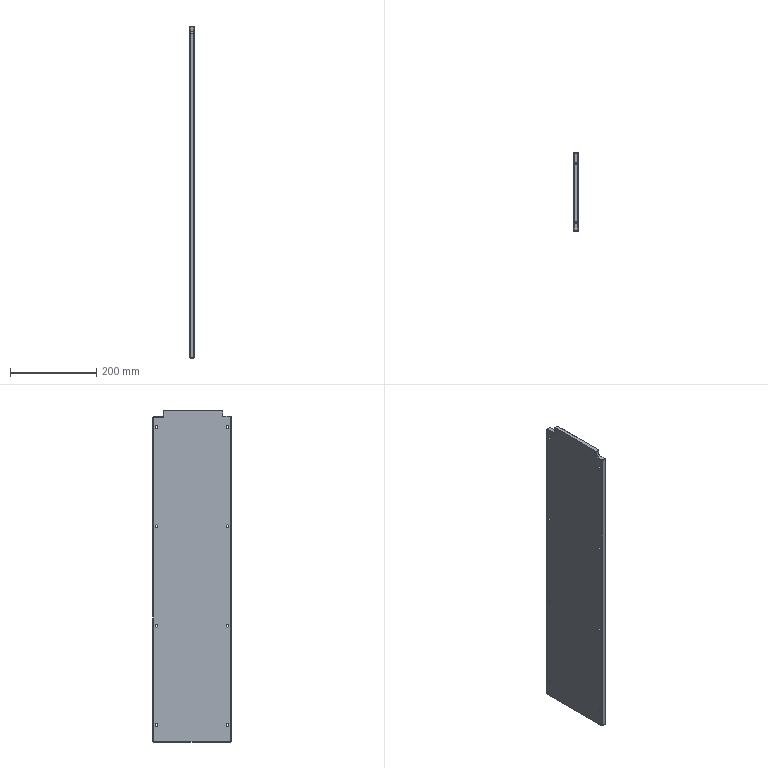Part | NX | 1 solid | 58 faces | box 10 x 182 x 768 mm | volume 1386280 mm3 | plane 26 | cylinder 16 | cone 16 | commonest cylinder face diameters 4 x8 6.5 x8
STEP:
#1=CARTESIAN_POINT('',(-4.,89.,-384.));
#2=VERTEX_POINT('',#1);
#3=CARTESIAN_POINT('',(4.,89.,-384.));
#4=VERTEX_POINT('',#3);
#5=CARTESIAN_POINT('',(5.,89.,-384.));
#6=DIRECTION('',(-1.,0.,0.));
#7=VECTOR('',#6,1000.);
#8=LINE('',#5,#7);
#9=EDGE_CURVE('',#2,#4,#8,.F.);
#10=ORIENTED_EDGE('',*,*,#9,.T.);
#11=CARTESIAN_POINT('',(4.,-89.,-384.));
#12=VERTEX_POINT('',#11);
#13=CARTESIAN_POINT('',(4.,-91.,-384.));
#14=DIRECTION('',(0.,-1.,0.));
#15=VECTOR('',#14,1000.);
#16=LINE('',#13,#15);
#17=EDGE_CURVE('',#4,#12,#16,.T.);
#18=ORIENTED_EDGE('',*,*,#17,.T.);
#19=CARTESIAN_POINT('',(-4.,-89.,-384.));
#20=VERTEX_POINT('',#19);
#21=CARTESIAN_POINT('',(5.,-89.,-384.));
#22=DIRECTION('',(-1.,0.,0.));
#23=VECTOR('',#22,1000.);
#24=LINE('',#21,#23);
#25=EDGE_CURVE('',#12,#20,#24,.T.);
#26=ORIENTED_EDGE('',*,*,#25,.T.);
#27=CARTESIAN_POINT('',(-4.,89.,-384.));
#28=DIRECTION('',(0.,1.,0.));
#29=VECTOR('',#28,1000.);
#30=LINE('',#27,#29);
#31=EDGE_CURVE('',#20,#2,#30,.T.);
#32=ORIENTED_EDGE('',*,*,#31,.T.);
#33=EDGE_LOOP('',(#10,#18,#26,#32));
#34=FACE_BOUND('',#33,.T.);
#35=CARTESIAN_POINT('',(5.,-91.,-384.));
#36=DIRECTION('',(0.,0.,1.));
#37=DIRECTION('',(1.,0.,0.));
#38=AXIS2_PLACEMENT_3D('',#35,#36,#37);
#39=PLANE('',#38);
#40=ADVANCED_FACE('',(#34),#39,.F.);
#41=CARTESIAN_POINT('',(-4.,91.,366.));
#42=VERTEX_POINT('',#41);
#43=CARTESIAN_POINT('',(4.,91.,366.));
#44=VERTEX_POINT('',#43);
#45=CARTESIAN_POINT('',(5.,91.,366.));
#46=DIRECTION('',(1.,0.,0.));
#47=VECTOR('',#46,1000.);
#48=LINE('',#45,#47);
#49=EDGE_CURVE('',#42,#44,#48,.T.);
#50=ORIENTED_EDGE('',*,*,#49,.T.);
#51=CARTESIAN_POINT('',(4.,91.,-382.));
#52=VERTEX_POINT('',#51);
#53=CARTESIAN_POINT('',(4.,91.,384.));
#54=DIRECTION('',(0.,0.,-1.));
#55=VECTOR('',#54,1000.);
#56=LINE('',#53,#55);
#57=EDGE_CURVE('',#44,#52,#56,.T.);
#58=ORIENTED_EDGE('',*,*,#57,.T.);
#59=CARTESIAN_POINT('',(-4.,91.,-382.));
#60=VERTEX_POINT('',#59);
#61=CARTESIAN_POINT('',(5.,91.,-382.));
#62=DIRECTION('',(-1.,0.,0.));
#63=VECTOR('',#62,1000.);
#64=LINE('',#61,#63);
#65=EDGE_CURVE('',#52,#60,#64,.T.);
#66=ORIENTED_EDGE('',*,*,#65,.T.);
#67=CARTESIAN_POINT('',(-4.,91.,366.));
#68=DIRECTION('',(0.,0.,1.));
#69=VECTOR('',#68,1000.);
#70=LINE('',#67,#69);
#71=EDGE_CURVE('',#60,#42,#70,.T.);
#72=ORIENTED_EDGE('',*,*,#71,.T.);
#73=EDGE_LOOP('',(#50,#58,#66,#72));
#74=FACE_BOUND('',#73,.T.);
#75=CARTESIAN_POINT('',(5.,91.,384.));
#76=DIRECTION('',(0.,-1.,0.));
#77=DIRECTION('',(0.,0.,-1.));
#78=AXIS2_PLACEMENT_3D('',#75,#76,#77);
#79=PLANE('',#78);
#80=ADVANCED_FACE('',(#74),#79,.F.);
#81=CARTESIAN_POINT('',(-4.,-69.,384.));
#82=VERTEX_POINT('',#81);
#83=CARTESIAN_POINT('',(4.,-69.,384.));
#84=VERTEX_POINT('',#83);
#85=CARTESIAN_POINT('',(5.,-69.,384.));
#86=DIRECTION('',(1.,0.,0.));
#87=VECTOR('',#86,1000.);
#88=LINE('',#85,#87);
#89=EDGE_CURVE('',#82,#84,#88,.T.);
#90=ORIENTED_EDGE('',*,*,#89,.T.);
#91=CARTESIAN_POINT('',(4.,64.,384.));
#92=VERTEX_POINT('',#91);
#93=CARTESIAN_POINT('',(4.,-91.,384.));
#94=DIRECTION('',(0.,1.,0.));
#95=VECTOR('',#94,1000.);
#96=LINE('',#93,#95);
#97=EDGE_CURVE('',#84,#92,#96,.T.);
#98=ORIENTED_EDGE('',*,*,#97,.T.);
#99=CARTESIAN_POINT('',(-4.,64.,384.));
#100=VERTEX_POINT('',#99);
#101=CARTESIAN_POINT('',(5.,64.,384.));
#102=DIRECTION('',(1.,0.,0.));
#103=VECTOR('',#102,1000.);
#104=LINE('',#101,#103);
#105=EDGE_CURVE('',#92,#100,#104,.F.);
#106=ORIENTED_EDGE('',*,*,#105,.T.);
#107=CARTESIAN_POINT('',(-4.,-69.,384.));
#108=DIRECTION('',(0.,-1.,0.));
#109=VECTOR('',#108,1000.);
#110=LINE('',#107,#109);
#111=EDGE_CURVE('',#100,#82,#110,.T.);
#112=ORIENTED_EDGE('',*,*,#111,.T.);
#113=EDGE_LOOP('',(#90,#98,#106,#112));
#114=FACE_BOUND('',#113,.T.);
#115=CARTESIAN_POINT('',(5.,-91.,384.));
#116=DIRECTION('',(0.,0.,-1.));
#117=DIRECTION('',(-1.,0.,0.));
#118=AXIS2_PLACEMENT_3D('',#115,#116,#117);
#119=PLANE('',#118);
#120=ADVANCED_FACE('',(#114),#119,.F.);
#121=CARTESIAN_POINT('',(-4.,-91.,-382.));
#122=VERTEX_POINT('',#121);
#123=CARTESIAN_POINT('',(4.,-91.,-382.));
#124=VERTEX_POINT('',#123);
#125=CARTESIAN_POINT('',(5.,-91.,-382.));
#126=DIRECTION('',(-1.,0.,0.));
#127=VECTOR('',#126,1000.);
#128=LINE('',#125,#127);
#129=EDGE_CURVE('',#122,#124,#128,.F.);
#130=ORIENTED_EDGE('',*,*,#129,.T.);
#131=CARTESIAN_POINT('',(4.,-91.,367.5));
#132=VERTEX_POINT('',#131);
#133=CARTESIAN_POINT('',(4.,-91.,384.));
#134=DIRECTION('',(0.,0.,1.));
#135=VECTOR('',#134,1000.);
#136=LINE('',#133,#135);
#137=EDGE_CURVE('',#124,#132,#136,.T.);
#138=ORIENTED_EDGE('',*,*,#137,.T.);
#139=CARTESIAN_POINT('',(-4.,-91.,367.5));
#140=VERTEX_POINT('',#139);
#141=CARTESIAN_POINT('',(5.,-91.,367.5));
#142=DIRECTION('',(1.,0.,0.));
#143=VECTOR('',#142,1000.);
#144=LINE('',#141,#143);
#145=EDGE_CURVE('',#132,#140,#144,.F.);
#146=ORIENTED_EDGE('',*,*,#145,.T.);
#147=CARTESIAN_POINT('',(-4.,-91.,-382.));
#148=DIRECTION('',(0.,0.,-1.));
#149=VECTOR('',#148,1000.);
#150=LINE('',#147,#149);
#151=EDGE_CURVE('',#140,#122,#150,.T.);
#152=ORIENTED_EDGE('',*,*,#151,.T.);
#153=EDGE_LOOP('',(#130,#138,#146,#152));
#154=FACE_BOUND('',#153,.T.);
#155=CARTESIAN_POINT('',(5.,-91.,384.));
#156=DIRECTION('',(0.,1.,0.));
#157=DIRECTION('',(0.,0.,1.));
#158=AXIS2_PLACEMENT_3D('',#155,#156,#157);
#159=PLANE('',#158);
#160=ADVANCED_FACE('',(#154),#159,.F.);
#161=CARTESIAN_POINT('',(5.,65.,370.));
#162=VERTEX_POINT('',#161);
#163=CARTESIAN_POINT('',(5.,65.,382.));
#164=VERTEX_POINT('',#163);
#165=CARTESIAN_POINT('',(5.,65.,0.));
#166=DIRECTION('',(0.,0.,1.));
#167=VECTOR('',#166,1000.);
#168=LINE('',#165,#167);
#169=EDGE_CURVE('',#162,#164,#168,.T.);
#170=ORIENTED_EDGE('',*,*,#169,.T.);
#171=CARTESIAN_POINT('',(5.,64.,383.));
#172=VERTEX_POINT('',#171);
#173=CARTESIAN_POINT('',(5.,64.,382.));
#174=DIRECTION('',(-1.,0.,0.));
#175=DIRECTION('',(0.,0.,1.));
#176=AXIS2_PLACEMENT_3D('',#173,#174,#175);
#177=CIRCLE('',#176,1.);
#178=EDGE_CURVE('',#164,#172,#177,.F.);
#179=ORIENTED_EDGE('',*,*,#178,.T.);
#180=CARTESIAN_POINT('',(5.,-69.,383.));
#181=VERTEX_POINT('',#180);
#182=CARTESIAN_POINT('',(5.,0.,383.));
#183=DIRECTION('',(0.,-1.,0.));
#184=VECTOR('',#183,1000.);
#185=LINE('',#182,#184);
#186=EDGE_CURVE('',#172,#181,#185,.T.);
#187=ORIENTED_EDGE('',*,*,#186,.T.);
#188=CARTESIAN_POINT('',(5.,-70.,382.));
#189=VERTEX_POINT('',#188);
#190=CARTESIAN_POINT('',(5.,-69.,382.));
#191=DIRECTION('',(-1.,0.,0.));
#192=DIRECTION('',(0.,0.,1.));
#193=AXIS2_PLACEMENT_3D('',#190,#191,#192);
#194=CIRCLE('',#193,1.);
#195=EDGE_CURVE('',#181,#189,#194,.F.);
#196=ORIENTED_EDGE('',*,*,#195,.T.);
#197=CARTESIAN_POINT('',(5.,-70.,371.5));
#198=VERTEX_POINT('',#197);
#199=CARTESIAN_POINT('',(5.,-70.,0.));
#200=DIRECTION('',(0.,0.,-1.));
#201=VECTOR('',#200,1000.);
#202=LINE('',#199,#201);
#203=EDGE_CURVE('',#189,#198,#202,.T.);
#204=ORIENTED_EDGE('',*,*,#203,.T.);
#205=CARTESIAN_POINT('',(5.,-73.,368.5));
#206=VERTEX_POINT('',#205);
#207=CARTESIAN_POINT('',(5.,-73.,371.5));
#208=DIRECTION('',(-1.,0.,0.));
#209=DIRECTION('',(0.,0.,1.));
#210=AXIS2_PLACEMENT_3D('',#207,#208,#209);
#211=CIRCLE('',#210,3.);
#212=EDGE_CURVE('',#198,#206,#211,.T.);
#213=ORIENTED_EDGE('',*,*,#212,.T.);
#214=CARTESIAN_POINT('',(5.,-89.,368.5));
#215=VERTEX_POINT('',#214);
#216=CARTESIAN_POINT('',(5.,0.,368.5));
#217=DIRECTION('',(0.,-1.,0.));
#218=VECTOR('',#217,1000.);
#219=LINE('',#216,#218);
#220=EDGE_CURVE('',#206,#215,#219,.T.);
#221=ORIENTED_EDGE('',*,*,#220,.T.);
#222=CARTESIAN_POINT('',(5.,-90.,367.5));
#223=VERTEX_POINT('',#222);
#224=CARTESIAN_POINT('',(5.,-89.,367.5));
#225=DIRECTION('',(-1.,0.,0.));
#226=DIRECTION('',(0.,0.,1.));
#227=AXIS2_PLACEMENT_3D('',#224,#225,#226);
#228=CIRCLE('',#227,1.);
#229=EDGE_CURVE('',#215,#223,#228,.F.);
#230=ORIENTED_EDGE('',*,*,#229,.T.);
#231=CARTESIAN_POINT('',(5.,-90.,-382.));
#232=VERTEX_POINT('',#231);
#233=CARTESIAN_POINT('',(5.,-90.,0.));
#234=DIRECTION('',(0.,0.,-1.));
#235=VECTOR('',#234,1000.);
#236=LINE('',#233,#235);
#237=EDGE_CURVE('',#223,#232,#236,.T.);
#238=ORIENTED_EDGE('',*,*,#237,.T.);
#239=CARTESIAN_POINT('',(5.,-89.,-383.));
#240=VERTEX_POINT('',#239);
#241=CARTESIAN_POINT('',(5.,-89.,-382.));
#242=DIRECTION('',(-1.,0.,0.));
#243=DIRECTION('',(0.,0.,1.));
#244=AXIS2_PLACEMENT_3D('',#241,#242,#243);
#245=CIRCLE('',#244,1.);
#246=EDGE_CURVE('',#232,#240,#245,.F.);
#247=ORIENTED_EDGE('',*,*,#246,.T.);
#248=CARTESIAN_POINT('',(5.,89.,-383.));
#249=VERTEX_POINT('',#248);
#250=CARTESIAN_POINT('',(5.,0.,-383.));
#251=DIRECTION('',(0.,1.,0.));
#252=VECTOR('',#251,1000.);
#253=LINE('',#250,#252);
#254=EDGE_CURVE('',#240,#249,#253,.T.);
#255=ORIENTED_EDGE('',*,*,#254,.T.);
#256=CARTESIAN_POINT('',(5.,90.,-382.));
#257=VERTEX_POINT('',#256);
#258=CARTESIAN_POINT('',(5.,89.,-382.));
#259=DIRECTION('',(-1.,0.,0.));
#260=DIRECTION('',(0.,0.,1.));
#261=AXIS2_PLACEMENT_3D('',#258,#259,#260);
#262=CIRCLE('',#261,1.);
#263=EDGE_CURVE('',#249,#257,#262,.F.);
#264=ORIENTED_EDGE('',*,*,#263,.T.);
#265=CARTESIAN_POINT('',(5.,90.,366.));
#266=VERTEX_POINT('',#265);
#267=CARTESIAN_POINT('',(5.,90.,0.));
#268=DIRECTION('',(0.,0.,1.));
#269=VECTOR('',#268,1000.);
#270=LINE('',#267,#269);
#271=EDGE_CURVE('',#257,#266,#270,.T.);
#272=ORIENTED_EDGE('',*,*,#271,.T.);
#273=CARTESIAN_POINT('',(5.,89.,367.));
#274=VERTEX_POINT('',#273);
#275=CARTESIAN_POINT('',(5.,89.,366.));
#276=DIRECTION('',(-1.,0.,0.));
#277=DIRECTION('',(0.,0.,1.));
#278=AXIS2_PLACEMENT_3D('',#275,#276,#277);
#279=CIRCLE('',#278,1.);
#280=EDGE_CURVE('',#266,#274,#279,.F.);
#281=ORIENTED_EDGE('',*,*,#280,.T.);
#282=CARTESIAN_POINT('',(5.,68.,367.));
#283=VERTEX_POINT('',#282);
#284=CARTESIAN_POINT('',(5.,0.,367.));
#285=DIRECTION('',(0.,-1.,0.));
#286=VECTOR('',#285,1000.);
#287=LINE('',#284,#286);
#288=EDGE_CURVE('',#274,#283,#287,.T.);
#289=ORIENTED_EDGE('',*,*,#288,.T.);
#290=CARTESIAN_POINT('',(5.,68.,370.));
#291=DIRECTION('',(-1.,0.,0.));
#292=DIRECTION('',(0.,0.,1.));
#293=AXIS2_PLACEMENT_3D('',#290,#291,#292);
#294=CIRCLE('',#293,3.);
#295=EDGE_CURVE('',#283,#162,#294,.T.);
#296=ORIENTED_EDGE('',*,*,#295,.T.);
#297=EDGE_LOOP('',(#170,#179,#187,#196,#204,#213,#221,#230,#238,#247,#255,#264,#272,#281,#289,#296));
#298=FACE_BOUND('',#297,.T.);
#299=CARTESIAN_POINT('',(5.,82.,-118.25));
#300=VERTEX_POINT('',#299);
#301=CARTESIAN_POINT('',(5.,82.,-115.));
#302=DIRECTION('',(1.,0.,0.));
#303=DIRECTION('',(0.,0.,-1.));
#304=AXIS2_PLACEMENT_3D('',#301,#302,#303);
#305=CIRCLE('',#304,3.25);
#306=EDGE_CURVE('',#300,#300,#305,.T.);
#307=ORIENTED_EDGE('',*,*,#306,.F.);
#308=EDGE_LOOP('',(#307));
#309=FACE_BOUND('',#308,.T.);
#310=CARTESIAN_POINT('',(5.,82.,-348.25));
#311=VERTEX_POINT('',#310);
#312=CARTESIAN_POINT('',(5.,82.,-345.));
#313=DIRECTION('',(1.,0.,0.));
#314=DIRECTION('',(0.,0.,-1.));
#315=AXIS2_PLACEMENT_3D('',#312,#313,#314);
#316=CIRCLE('',#315,3.25);
#317=EDGE_CURVE('',#311,#311,#316,.T.);
#318=ORIENTED_EDGE('',*,*,#317,.F.);
#319=EDGE_LOOP('',(#318));
#320=FACE_BOUND('',#319,.T.);
#321=CARTESIAN_POINT('',(5.,82.,341.75));
#322=VERTEX_POINT('',#321);
#323=CARTESIAN_POINT('',(5.,82.,345.));
#324=DIRECTION('',(1.,0.,0.));
#325=DIRECTION('',(0.,0.,-1.));
#326=AXIS2_PLACEMENT_3D('',#323,#324,#325);
#327=CIRCLE('',#326,3.25);
#328=EDGE_CURVE('',#322,#322,#327,.T.);
#329=ORIENTED_EDGE('',*,*,#328,.F.);
#330=EDGE_LOOP('',(#329));
#331=FACE_BOUND('',#330,.T.);
#332=CARTESIAN_POINT('',(5.,82.,111.75));
#333=VERTEX_POINT('',#332);
#334=CARTESIAN_POINT('',(5.,82.,115.));
#335=DIRECTION('',(1.,0.,0.));
#336=DIRECTION('',(0.,0.,-1.));
#337=AXIS2_PLACEMENT_3D('',#334,#335,#336);
#338=CIRCLE('',#337,3.25);
#339=EDGE_CURVE('',#333,#333,#338,.T.);
#340=ORIENTED_EDGE('',*,*,#339,.F.);
#341=EDGE_LOOP('',(#340));
#342=FACE_BOUND('',#341,.T.);
#343=CARTESIAN_POINT('',(5.,-82.,341.75));
#344=VERTEX_POINT('',#343);
#345=CARTESIAN_POINT('',(5.,-82.,345.));
#346=DIRECTION('',(1.,0.,0.));
#347=DIRECTION('',(0.,0.,-1.));
#348=AXIS2_PLACEMENT_3D('',#345,#346,#347);
#349=CIRCLE('',#348,3.25);
#350=EDGE_CURVE('',#344,#344,#349,.T.);
#351=ORIENTED_EDGE('',*,*,#350,.F.);
#352=EDGE_LOOP('',(#351));
#353=FACE_BOUND('',#352,.T.);
#354=CARTESIAN_POINT('',(5.,-82.,111.75));
#355=VERTEX_POINT('',#354);
#356=CARTESIAN_POINT('',(5.,-82.,115.));
#357=DIRECTION('',(1.,0.,0.));
#358=DIRECTION('',(0.,0.,-1.));
#359=AXIS2_PLACEMENT_3D('',#356,#357,#358);
#360=CIRCLE('',#359,3.25);
#361=EDGE_CURVE('',#355,#355,#360,.T.);
#362=ORIENTED_EDGE('',*,*,#361,.F.);
#363=EDGE_LOOP('',(#362));
#364=FACE_BOUND('',#363,.T.);
#365=CARTESIAN_POINT('',(5.,-82.,-118.25));
#366=VERTEX_POINT('',#365);
#367=CARTESIAN_POINT('',(5.,-82.,-115.));
#368=DIRECTION('',(1.,0.,0.));
#369=DIRECTION('',(0.,0.,-1.));
#370=AXIS2_PLACEMENT_3D('',#367,#368,#369);
#371=CIRCLE('',#370,3.25);
#372=EDGE_CURVE('',#366,#366,#371,.T.);
#373=ORIENTED_EDGE('',*,*,#372,.F.);
#374=EDGE_LOOP('',(#373));
#375=FACE_BOUND('',#374,.T.);
#376=CARTESIAN_POINT('',(5.,-82.,-348.25));
#377=VERTEX_POINT('',#376);
#378=CARTESIAN_POINT('',(5.,-82.,-345.));
#379=DIRECTION('',(1.,0.,0.));
#380=DIRECTION('',(0.,0.,-1.));
#381=AXIS2_PLACEMENT_3D('',#378,#379,#380);
#382=CIRCLE('',#381,3.25);
#383=EDGE_CURVE('',#377,#377,#382,.T.);
#384=ORIENTED_EDGE('',*,*,#383,.F.);
#385=EDGE_LOOP('',(#384));
#386=FACE_BOUND('',#385,.T.);
#387=CARTESIAN_POINT('',(5.,0.,0.));
#388=DIRECTION('',(-1.,0.,0.));
#389=DIRECTION('',(0.,0.,1.));
#390=AXIS2_PLACEMENT_3D('',#387,#388,#389);
#391=PLANE('',#390);
#392=ADVANCED_FACE('',(#298,#309,#320,#331,#342,#353,#364,#375,#386),#391,.F.);
#393=CARTESIAN_POINT('',(-5.,90.,-382.));
#394=VERTEX_POINT('',#393);
#395=CARTESIAN_POINT('',(-5.,89.,-383.));
#396=VERTEX_POINT('',#395);
#397=CARTESIAN_POINT('',(-5.,89.,-382.));
#398=DIRECTION('',(-1.,0.,0.));
#399=DIRECTION('',(0.,0.,1.));
#400=AXIS2_PLACEMENT_3D('',#397,#398,#399);
#401=CIRCLE('',#400,1.);
#402=EDGE_CURVE('',#394,#396,#401,.T.);
#403=ORIENTED_EDGE('',*,*,#402,.T.);
#404=CARTESIAN_POINT('',(-5.,-89.,-383.));
#405=VERTEX_POINT('',#404);
#406=CARTESIAN_POINT('',(-5.,-89.,-383.));
#407=DIRECTION('',(0.,-1.,0.));
#408=VECTOR('',#407,1000.);
#409=LINE('',#406,#408);
#410=EDGE_CURVE('',#396,#405,#409,.T.);
#411=ORIENTED_EDGE('',*,*,#410,.T.);
#412=CARTESIAN_POINT('',(-5.,-90.,-382.));
#413=VERTEX_POINT('',#412);
#414=CARTESIAN_POINT('',(-5.,-89.,-382.));
#415=DIRECTION('',(-1.,0.,0.));
#416=DIRECTION('',(0.,0.,1.));
#417=AXIS2_PLACEMENT_3D('',#414,#415,#416);
#418=CIRCLE('',#417,1.);
#419=EDGE_CURVE('',#405,#413,#418,.T.);
#420=ORIENTED_EDGE('',*,*,#419,.T.);
#421=CARTESIAN_POINT('',(-5.,-90.,367.5));
#422=VERTEX_POINT('',#421);
#423=CARTESIAN_POINT('',(-5.,-90.,367.5));
#424=DIRECTION('',(0.,0.,1.));
#425=VECTOR('',#424,1000.);
#426=LINE('',#423,#425);
#427=EDGE_CURVE('',#413,#422,#426,.T.);
#428=ORIENTED_EDGE('',*,*,#427,.T.);
#429=CARTESIAN_POINT('',(-5.,-89.,368.5));
#430=VERTEX_POINT('',#429);
#431=CARTESIAN_POINT('',(-5.,-89.,367.5));
#432=DIRECTION('',(-1.,0.,0.));
#433=DIRECTION('',(0.,0.,1.));
#434=AXIS2_PLACEMENT_3D('',#431,#432,#433);
#435=CIRCLE('',#434,1.);
#436=EDGE_CURVE('',#422,#430,#435,.T.);
#437=ORIENTED_EDGE('',*,*,#436,.T.);
#438=CARTESIAN_POINT('',(-5.,-73.,368.5));
#439=VERTEX_POINT('',#438);
#440=CARTESIAN_POINT('',(-5.,-73.,368.5));
#441=DIRECTION('',(0.,1.,0.));
#442=VECTOR('',#441,1000.);
#443=LINE('',#440,#442);
#444=EDGE_CURVE('',#430,#439,#443,.T.);
#445=ORIENTED_EDGE('',*,*,#444,.T.);
#446=CARTESIAN_POINT('',(-5.,-70.,371.5));
#447=VERTEX_POINT('',#446);
#448=CARTESIAN_POINT('',(-5.,-73.,371.5));
#449=DIRECTION('',(-1.,0.,0.));
#450=DIRECTION('',(0.,0.,1.));
#451=AXIS2_PLACEMENT_3D('',#448,#449,#450);
#452=CIRCLE('',#451,3.);
#453=EDGE_CURVE('',#439,#447,#452,.F.);
#454=ORIENTED_EDGE('',*,*,#453,.T.);
#455=CARTESIAN_POINT('',(-5.,-70.,382.));
#456=VERTEX_POINT('',#455);
#457=CARTESIAN_POINT('',(-5.,-70.,382.));
#458=DIRECTION('',(0.,0.,1.));
#459=VECTOR('',#458,1000.);
#460=LINE('',#457,#459);
#461=EDGE_CURVE('',#447,#456,#460,.T.);
#462=ORIENTED_EDGE('',*,*,#461,.T.);
#463=CARTESIAN_POINT('',(-5.,-69.,383.));
#464=VERTEX_POINT('',#463);
#465=CARTESIAN_POINT('',(-5.,-69.,382.));
#466=DIRECTION('',(-1.,0.,0.));
#467=DIRECTION('',(0.,0.,1.));
#468=AXIS2_PLACEMENT_3D('',#465,#466,#467);
#469=CIRCLE('',#468,1.);
#470=EDGE_CURVE('',#456,#464,#469,.T.);
#471=ORIENTED_EDGE('',*,*,#470,.T.);
#472=CARTESIAN_POINT('',(-5.,64.,383.));
#473=VERTEX_POINT('',#472);
#474=CARTESIAN_POINT('',(-5.,64.,383.));
#475=DIRECTION('',(0.,1.,0.));
#476=VECTOR('',#475,1000.);
#477=LINE('',#474,#476);
#478=EDGE_CURVE('',#464,#473,#477,.T.);
#479=ORIENTED_EDGE('',*,*,#478,.T.);
#480=CARTESIAN_POINT('',(-5.,65.,382.));
#481=VERTEX_POINT('',#480);
#482=CARTESIAN_POINT('',(-5.,64.,382.));
#483=DIRECTION('',(-1.,0.,0.));
#484=DIRECTION('',(0.,0.,1.));
#485=AXIS2_PLACEMENT_3D('',#482,#483,#484);
#486=CIRCLE('',#485,1.);
#487=EDGE_CURVE('',#473,#481,#486,.T.);
#488=ORIENTED_EDGE('',*,*,#487,.T.);
#489=CARTESIAN_POINT('',(-5.,65.,370.));
#490=VERTEX_POINT('',#489);
#491=CARTESIAN_POINT('',(-5.,65.,370.));
#492=DIRECTION('',(0.,0.,-1.));
#493=VECTOR('',#492,1000.);
#494=LINE('',#491,#493);
#495=EDGE_CURVE('',#481,#490,#494,.T.);
#496=ORIENTED_EDGE('',*,*,#495,.T.);
#497=CARTESIAN_POINT('',(-5.,68.,367.));
#498=VERTEX_POINT('',#497);
#499=CARTESIAN_POINT('',(-5.,68.,370.));
#500=DIRECTION('',(-1.,0.,0.));
#501=DIRECTION('',(0.,0.,1.));
#502=AXIS2_PLACEMENT_3D('',#499,#500,#501);
#503=CIRCLE('',#502,3.);
#504=EDGE_CURVE('',#490,#498,#503,.F.);
#505=ORIENTED_EDGE('',*,*,#504,.T.);
#506=CARTESIAN_POINT('',(-5.,89.,367.));
#507=VERTEX_POINT('',#506);
#508=CARTESIAN_POINT('',(-5.,89.,367.));
#509=DIRECTION('',(0.,1.,0.));
#510=VECTOR('',#509,1000.);
#511=LINE('',#508,#510);
#512=EDGE_CURVE('',#498,#507,#511,.T.);
#513=ORIENTED_EDGE('',*,*,#512,.T.);
#514=CARTESIAN_POINT('',(-5.,90.,366.));
#515=VERTEX_POINT('',#514);
#516=CARTESIAN_POINT('',(-5.,89.,366.));
#517=DIRECTION('',(-1.,0.,0.));
#518=DIRECTION('',(0.,0.,1.));
#519=AXIS2_PLACEMENT_3D('',#516,#517,#518);
#520=CIRCLE('',#519,1.);
#521=EDGE_CURVE('',#507,#515,#520,.T.);
#522=ORIENTED_EDGE('',*,*,#521,.T.);
#523=CARTESIAN_POINT('',(-5.,90.,-382.));
#524=DIRECTION('',(0.,0.,-1.));
#525=VECTOR('',#524,1000.);
#526=LINE('',#523,#525);
#527=EDGE_CURVE('',#515,#394,#526,.T.);
#528=ORIENTED_EDGE('',*,*,#527,.T.);
#529=EDGE_LOOP('',(#403,#411,#420,#428,#437,#445,#454,#462,#471,#479,#488,#496,#505,#513,#522,#528));
#530=FACE_BOUND('',#529,.T.);
#531=CARTESIAN_POINT('',(-5.,82.,-118.25));
#532=VERTEX_POINT('',#531);
#533=CARTESIAN_POINT('',(-5.,82.,-115.));
#534=DIRECTION('',(1.,0.,0.));
#535=DIRECTION('',(0.,0.,-1.));
#536=AXIS2_PLACEMENT_3D('',#533,#534,#535);
#537=CIRCLE('',#536,3.25);
#538=EDGE_CURVE('',#532,#532,#537,.T.);
#539=ORIENTED_EDGE('',*,*,#538,.T.);
#540=EDGE_LOOP('',(#539));
#541=FACE_BOUND('',#540,.T.);
#542=CARTESIAN_POINT('',(-5.,82.,-348.25));
#543=VERTEX_POINT('',#542);
#544=CARTESIAN_POINT('',(-5.,82.,-345.));
#545=DIRECTION('',(1.,0.,0.));
#546=DIRECTION('',(0.,0.,-1.));
#547=AXIS2_PLACEMENT_3D('',#544,#545,#546);
#548=CIRCLE('',#547,3.25);
#549=EDGE_CURVE('',#543,#543,#548,.T.);
#550=ORIENTED_EDGE('',*,*,#549,.T.);
#551=EDGE_LOOP('',(#550));
#552=FACE_BOUND('',#551,.T.);
#553=CARTESIAN_POINT('',(-5.,82.,341.75));
#554=VERTEX_POINT('',#553);
#555=CARTESIAN_POINT('',(-5.,82.,345.));
#556=DIRECTION('',(1.,0.,0.));
#557=DIRECTION('',(0.,0.,-1.));
#558=AXIS2_PLACEMENT_3D('',#555,#556,#557);
#559=CIRCLE('',#558,3.25);
#560=EDGE_CURVE('',#554,#554,#559,.T.);
#561=ORIENTED_EDGE('',*,*,#560,.T.);
#562=EDGE_LOOP('',(#561));
#563=FACE_BOUND('',#562,.T.);
#564=CARTESIAN_POINT('',(-5.,82.,111.75));
#565=VERTEX_POINT('',#564);
#566=CARTESIAN_POINT('',(-5.,82.,115.));
#567=DIRECTION('',(1.,0.,0.));
#568=DIRECTION('',(0.,0.,-1.));
#569=AXIS2_PLACEMENT_3D('',#566,#567,#568);
#570=CIRCLE('',#569,3.25);
#571=EDGE_CURVE('',#565,#565,#570,.T.);
#572=ORIENTED_EDGE('',*,*,#571,.T.);
#573=EDGE_LOOP('',(#572));
#574=FACE_BOUND('',#573,.T.);
#575=CARTESIAN_POINT('',(-5.,-82.,341.75));
#576=VERTEX_POINT('',#575);
#577=CARTESIAN_POINT('',(-5.,-82.,345.));
#578=DIRECTION('',(1.,0.,0.));
#579=DIRECTION('',(0.,0.,-1.));
#580=AXIS2_PLACEMENT_3D('',#577,#578,#579);
#581=CIRCLE('',#580,3.25);
#582=EDGE_CURVE('',#576,#576,#581,.T.);
#583=ORIENTED_EDGE('',*,*,#582,.T.);
#584=EDGE_LOOP('',(#583));
#585=FACE_BOUND('',#584,.T.);
#586=CARTESIAN_POINT('',(-5.,-82.,111.75));
#587=VERTEX_POINT('',#586);
#588=CARTESIAN_POINT('',(-5.,-82.,115.));
#589=DIRECTION('',(1.,0.,0.));
#590=DIRECTION('',(0.,0.,-1.));
#591=AXIS2_PLACEMENT_3D('',#588,#589,#590);
#592=CIRCLE('',#591,3.25);
#593=EDGE_CURVE('',#587,#587,#592,.T.);
#594=ORIENTED_EDGE('',*,*,#593,.T.);
#595=EDGE_LOOP('',(#594));
#596=FACE_BOUND('',#595,.T.);
#597=CARTESIAN_POINT('',(-5.,-82.,-118.25));
#598=VERTEX_POINT('',#597);
#599=CARTESIAN_POINT('',(-5.,-82.,-115.));
#600=DIRECTION('',(1.,0.,0.));
#601=DIRECTION('',(0.,0.,-1.));
#602=AXIS2_PLACEMENT_3D('',#599,#600,#601);
#603=CIRCLE('',#602,3.25);
#604=EDGE_CURVE('',#598,#598,#603,.T.);
#605=ORIENTED_EDGE('',*,*,#604,.T.);
#606=EDGE_LOOP('',(#605));
#607=FACE_BOUND('',#606,.T.);
#608=CARTESIAN_POINT('',(-5.,-82.,-348.25));
#609=VERTEX_POINT('',#608);
#610=CARTESIAN_POINT('',(-5.,-82.,-345.));
#611=DIRECTION('',(1.,0.,0.));
#612=DIRECTION('',(0.,0.,-1.));
#613=AXIS2_PLACEMENT_3D('',#610,#611,#612);
#614=CIRCLE('',#613,3.25);
#615=EDGE_CURVE('',#609,#609,#614,.T.);
#616=ORIENTED_EDGE('',*,*,#615,.T.);
#617=EDGE_LOOP('',(#616));
#618=FACE_BOUND('',#617,.T.);
#619=CARTESIAN_POINT('',(-5.,0.,0.));
#620=DIRECTION('',(-1.,0.,0.));
#621=DIRECTION('',(0.,0.,1.));
#622=AXIS2_PLACEMENT_3D('',#619,#620,#621);
#623=PLANE('',#622);
#624=ADVANCED_FACE('',(#530,#541,#552,#563,#574,#585,#596,#607,#618),#623,.T.);
#625=ORIENTED_EDGE('',*,*,#615,.F.);
#626=EDGE_LOOP('',(#625));
#627=FACE_BOUND('',#626,.T.);
#628=ORIENTED_EDGE('',*,*,#383,.T.);
#629=EDGE_LOOP('',(#628));
#630=FACE_BOUND('',#629,.T.);
#631=CARTESIAN_POINT('',(5.,-82.,-345.));
#632=DIRECTION('',(1.,0.,0.));
#633=DIRECTION('',(0.,0.,-1.));
#634=AXIS2_PLACEMENT_3D('',#631,#632,#633);
#635=CYLINDRICAL_SURFACE('',#634,3.25);
#636=ADVANCED_FACE('',(#627,#630),#635,.F.);
#637=ORIENTED_EDGE('',*,*,#604,.F.);
#638=EDGE_LOOP('',(#637));
#639=FACE_BOUND('',#638,.T.);
#640=ORIENTED_EDGE('',*,*,#372,.T.);
#641=EDGE_LOOP('',(#640));
#642=FACE_BOUND('',#641,.T.);
#643=CARTESIAN_POINT('',(5.,-82.,-115.));
#644=DIRECTION('',(1.,0.,0.));
#645=DIRECTION('',(0.,0.,-1.));
#646=AXIS2_PLACEMENT_3D('',#643,#644,#645);
#647=CYLINDRICAL_SURFACE('',#646,3.25);
#648=ADVANCED_FACE('',(#639,#642),#647,.F.);
#649=ORIENTED_EDGE('',*,*,#593,.F.);
#650=EDGE_LOOP('',(#649));
#651=FACE_BOUND('',#650,.T.);
#652=ORIENTED_EDGE('',*,*,#361,.T.);
#653=EDGE_LOOP('',(#652));
#654=FACE_BOUND('',#653,.T.);
#655=CARTESIAN_POINT('',(5.,-82.,115.));
#656=DIRECTION('',(1.,0.,0.));
#657=DIRECTION('',(0.,0.,-1.));
#658=AXIS2_PLACEMENT_3D('',#655,#656,#657);
#659=CYLINDRICAL_SURFACE('',#658,3.25);
#660=ADVANCED_FACE('',(#651,#654),#659,.F.);
#661=ORIENTED_EDGE('',*,*,#582,.F.);
#662=EDGE_LOOP('',(#661));
#663=FACE_BOUND('',#662,.T.);
#664=ORIENTED_EDGE('',*,*,#350,.T.);
#665=EDGE_LOOP('',(#664));
#666=FACE_BOUND('',#665,.T.);
#667=CARTESIAN_POINT('',(5.,-82.,345.));
#668=DIRECTION('',(1.,0.,0.));
#669=DIRECTION('',(0.,0.,-1.));
#670=AXIS2_PLACEMENT_3D('',#667,#668,#669);
#671=CYLINDRICAL_SURFACE('',#670,3.25);
#672=ADVANCED_FACE('',(#663,#666),#671,.F.);
#673=ORIENTED_EDGE('',*,*,#571,.F.);
#674=EDGE_LOOP('',(#673));
#675=FACE_BOUND('',#674,.T.);
#676=ORIENTED_EDGE('',*,*,#339,.T.);
#677=EDGE_LOOP('',(#676));
#678=FACE_BOUND('',#677,.T.);
#679=CARTESIAN_POINT('',(5.,82.,115.));
#680=DIRECTION('',(1.,0.,0.));
#681=DIRECTION('',(0.,0.,-1.));
#682=AXIS2_PLACEMENT_3D('',#679,#680,#681);
#683=CYLINDRICAL_SURFACE('',#682,3.25);
#684=ADVANCED_FACE('',(#675,#678),#683,.F.);
#685=ORIENTED_EDGE('',*,*,#560,.F.);
#686=EDGE_LOOP('',(#685));
#687=FACE_BOUND('',#686,.T.);
#688=ORIENTED_EDGE('',*,*,#328,.T.);
#689=EDGE_LOOP('',(#688));
#690=FACE_BOUND('',#689,.T.);
#691=CARTESIAN_POINT('',(5.,82.,345.));
#692=DIRECTION('',(1.,0.,0.));
#693=DIRECTION('',(0.,0.,-1.));
#694=AXIS2_PLACEMENT_3D('',#691,#692,#693);
#695=CYLINDRICAL_SURFACE('',#694,3.25);
#696=ADVANCED_FACE('',(#687,#690),#695,.F.);
#697=ORIENTED_EDGE('',*,*,#549,.F.);
#698=EDGE_LOOP('',(#697));
#699=FACE_BOUND('',#698,.T.);
#700=ORIENTED_EDGE('',*,*,#317,.T.);
#701=EDGE_LOOP('',(#700));
#702=FACE_BOUND('',#701,.T.);
#703=CARTESIAN_POINT('',(5.,82.,-345.));
#704=DIRECTION('',(1.,0.,0.));
#705=DIRECTION('',(0.,0.,-1.));
#706=AXIS2_PLACEMENT_3D('',#703,#704,#705);
#707=CYLINDRICAL_SURFACE('',#706,3.25);
#708=ADVANCED_FACE('',(#699,#702),#707,.F.);
#709=ORIENTED_EDGE('',*,*,#538,.F.);
#710=EDGE_LOOP('',(#709));
#711=FACE_BOUND('',#710,.T.);
#712=ORIENTED_EDGE('',*,*,#306,.T.);
#713=EDGE_LOOP('',(#712));
#714=FACE_BOUND('',#713,.T.);
#715=CARTESIAN_POINT('',(5.,82.,-115.));
#716=DIRECTION('',(1.,0.,0.));
#717=DIRECTION('',(0.,0.,-1.));
#718=AXIS2_PLACEMENT_3D('',#715,#716,#717);
#719=CYLINDRICAL_SURFACE('',#718,3.25);
#720=ADVANCED_FACE('',(#711,#714),#719,.F.);
#721=ORIENTED_EDGE('',*,*,#65,.F.);
#722=CARTESIAN_POINT('',(4.,89.,-382.));
#723=DIRECTION('',(-1.,0.,0.));
#724=DIRECTION('',(0.,0.,1.));
#725=AXIS2_PLACEMENT_3D('',#722,#723,#724);
#726=CIRCLE('',#725,2.);
#727=EDGE_CURVE('',#52,#4,#726,.T.);
#728=ORIENTED_EDGE('',*,*,#727,.T.);
#729=ORIENTED_EDGE('',*,*,#9,.F.);
#730=CARTESIAN_POINT('',(-4.,89.,-382.));
#731=DIRECTION('',(-1.,0.,0.));
#732=DIRECTION('',(0.,0.,1.));
#733=AXIS2_PLACEMENT_3D('',#730,#731,#732);
#734=CIRCLE('',#733,2.);
#735=EDGE_CURVE('',#2,#60,#734,.F.);
#736=ORIENTED_EDGE('',*,*,#735,.T.);
#737=EDGE_LOOP('',(#721,#728,#729,#736));
#738=FACE_BOUND('',#737,.T.);
#739=CARTESIAN_POINT('',(5.,89.,-382.));
#740=DIRECTION('',(-1.,0.,0.));
#741=DIRECTION('',(0.,0.,1.));
#742=AXIS2_PLACEMENT_3D('',#739,#740,#741);
#743=CYLINDRICAL_SURFACE('',#742,2.);
#744=ADVANCED_FACE('',(#738),#743,.T.);
#745=ORIENTED_EDGE('',*,*,#25,.F.);
#746=CARTESIAN_POINT('',(4.,-89.,-382.));
#747=DIRECTION('',(-1.,0.,0.));
#748=DIRECTION('',(0.,0.,1.));
#749=AXIS2_PLACEMENT_3D('',#746,#747,#748);
#750=CIRCLE('',#749,2.);
#751=EDGE_CURVE('',#12,#124,#750,.T.);
#752=ORIENTED_EDGE('',*,*,#751,.T.);
#753=ORIENTED_EDGE('',*,*,#129,.F.);
#754=CARTESIAN_POINT('',(-4.,-89.,-382.));
#755=DIRECTION('',(-1.,0.,0.));
#756=DIRECTION('',(0.,0.,1.));
#757=AXIS2_PLACEMENT_3D('',#754,#755,#756);
#758=CIRCLE('',#757,2.);
#759=EDGE_CURVE('',#122,#20,#758,.F.);
#760=ORIENTED_EDGE('',*,*,#759,.T.);
#761=EDGE_LOOP('',(#745,#752,#753,#760));
#762=FACE_BOUND('',#761,.T.);
#763=CARTESIAN_POINT('',(5.,-89.,-382.));
#764=DIRECTION('',(-1.,0.,0.));
#765=DIRECTION('',(0.,0.,1.));
#766=AXIS2_PLACEMENT_3D('',#763,#764,#765);
#767=CYLINDRICAL_SURFACE('',#766,2.);
#768=ADVANCED_FACE('',(#762),#767,.T.);
#769=CARTESIAN_POINT('',(-4.,-89.,369.5));
#770=VERTEX_POINT('',#769);
#771=CARTESIAN_POINT('',(4.,-89.,369.5));
#772=VERTEX_POINT('',#771);
#773=CARTESIAN_POINT('',(-5.,-89.,369.5));
#774=DIRECTION('',(1.,0.,0.));
#775=VECTOR('',#774,1000.);
#776=LINE('',#773,#775);
#777=EDGE_CURVE('',#770,#772,#776,.T.);
#778=ORIENTED_EDGE('',*,*,#777,.T.);
#779=CARTESIAN_POINT('',(4.,-73.,369.5));
#780=VERTEX_POINT('',#779);
#781=CARTESIAN_POINT('',(4.,-71.,369.5));
#782=DIRECTION('',(0.,1.,0.));
#783=VECTOR('',#782,1000.);
#784=LINE('',#781,#783);
#785=EDGE_CURVE('',#772,#780,#784,.T.);
#786=ORIENTED_EDGE('',*,*,#785,.T.);
#787=CARTESIAN_POINT('',(-4.,-73.,369.5));
#788=VERTEX_POINT('',#787);
#789=CARTESIAN_POINT('',(-5.,-73.,369.5));
#790=DIRECTION('',(1.,0.,0.));
#791=VECTOR('',#790,1000.);
#792=LINE('',#789,#791);
#793=EDGE_CURVE('',#780,#788,#792,.F.);
#794=ORIENTED_EDGE('',*,*,#793,.T.);
#795=CARTESIAN_POINT('',(-4.,-89.,369.5));
#796=DIRECTION('',(0.,-1.,0.));
#797=VECTOR('',#796,1000.);
#798=LINE('',#795,#797);
#799=EDGE_CURVE('',#788,#770,#798,.T.);
#800=ORIENTED_EDGE('',*,*,#799,.T.);
#801=EDGE_LOOP('',(#778,#786,#794,#800));
#802=FACE_BOUND('',#801,.T.);
#803=CARTESIAN_POINT('',(-5.,-71.,369.5));
#804=DIRECTION('',(0.,0.,-1.));
#805=DIRECTION('',(-1.,0.,0.));
#806=AXIS2_PLACEMENT_3D('',#803,#804,#805);
#807=PLANE('',#806);
#808=ADVANCED_FACE('',(#802),#807,.F.);
#809=CARTESIAN_POINT('',(-4.,-71.,371.5));
#810=VERTEX_POINT('',#809);
#811=CARTESIAN_POINT('',(4.,-71.,371.5));
#812=VERTEX_POINT('',#811);
#813=CARTESIAN_POINT('',(5.,-71.,371.5));
#814=DIRECTION('',(1.,0.,0.));
#815=VECTOR('',#814,1000.);
#816=LINE('',#813,#815);
#817=EDGE_CURVE('',#810,#812,#816,.T.);
#818=ORIENTED_EDGE('',*,*,#817,.T.);
#819=CARTESIAN_POINT('',(4.,-71.,382.));
#820=VERTEX_POINT('',#819);
#821=CARTESIAN_POINT('',(4.,-71.,369.5));
#822=DIRECTION('',(0.,0.,1.));
#823=VECTOR('',#822,1000.);
#824=LINE('',#821,#823);
#825=EDGE_CURVE('',#812,#820,#824,.T.);
#826=ORIENTED_EDGE('',*,*,#825,.T.);
#827=CARTESIAN_POINT('',(-4.,-71.,382.));
#828=VERTEX_POINT('',#827);
#829=CARTESIAN_POINT('',(-5.,-71.,382.));
#830=DIRECTION('',(1.,0.,0.));
#831=VECTOR('',#830,1000.);
#832=LINE('',#829,#831);
#833=EDGE_CURVE('',#820,#828,#832,.F.);
#834=ORIENTED_EDGE('',*,*,#833,.T.);
#835=CARTESIAN_POINT('',(-4.,-71.,371.5));
#836=DIRECTION('',(0.,0.,-1.));
#837=VECTOR('',#836,1000.);
#838=LINE('',#835,#837);
#839=EDGE_CURVE('',#828,#810,#838,.T.);
#840=ORIENTED_EDGE('',*,*,#839,.T.);
#841=EDGE_LOOP('',(#818,#826,#834,#840));
#842=FACE_BOUND('',#841,.T.);
#843=CARTESIAN_POINT('',(-5.,-71.,369.5));
#844=DIRECTION('',(0.,1.,0.));
#845=DIRECTION('',(0.,0.,1.));
#846=AXIS2_PLACEMENT_3D('',#843,#844,#845);
#847=PLANE('',#846);
#848=ADVANCED_FACE('',(#842),#847,.F.);
#849=CARTESIAN_POINT('',(-4.,68.,368.));
#850=VERTEX_POINT('',#849);
#851=CARTESIAN_POINT('',(4.,68.,368.));
#852=VERTEX_POINT('',#851);
#853=CARTESIAN_POINT('',(5.,68.,368.));
#854=DIRECTION('',(1.,0.,0.));
#855=VECTOR('',#854,1000.);
#856=LINE('',#853,#855);
#857=EDGE_CURVE('',#850,#852,#856,.T.);
#858=ORIENTED_EDGE('',*,*,#857,.T.);
#859=CARTESIAN_POINT('',(4.,89.,368.));
#860=VERTEX_POINT('',#859);
#861=CARTESIAN_POINT('',(4.,91.,368.));
#862=DIRECTION('',(0.,1.,0.));
#863=VECTOR('',#862,1000.);
#864=LINE('',#861,#863);
#865=EDGE_CURVE('',#852,#860,#864,.T.);
#866=ORIENTED_EDGE('',*,*,#865,.T.);
#867=CARTESIAN_POINT('',(-4.,89.,368.));
#868=VERTEX_POINT('',#867);
#869=CARTESIAN_POINT('',(-5.,89.,368.));
#870=DIRECTION('',(1.,0.,0.));
#871=VECTOR('',#870,1000.);
#872=LINE('',#869,#871);
#873=EDGE_CURVE('',#860,#868,#872,.F.);
#874=ORIENTED_EDGE('',*,*,#873,.T.);
#875=CARTESIAN_POINT('',(-4.,68.,368.));
#876=DIRECTION('',(0.,-1.,0.));
#877=VECTOR('',#876,1000.);
#878=LINE('',#875,#877);
#879=EDGE_CURVE('',#868,#850,#878,.T.);
#880=ORIENTED_EDGE('',*,*,#879,.T.);
#881=EDGE_LOOP('',(#858,#866,#874,#880));
#882=FACE_BOUND('',#881,.T.);
#883=CARTESIAN_POINT('',(-5.,91.,368.));
#884=DIRECTION('',(0.,0.,-1.));
#885=DIRECTION('',(-1.,0.,0.));
#886=AXIS2_PLACEMENT_3D('',#883,#884,#885);
#887=PLANE('',#886);
#888=ADVANCED_FACE('',(#882),#887,.F.);
#889=CARTESIAN_POINT('',(-4.,66.,382.));
#890=VERTEX_POINT('',#889);
#891=CARTESIAN_POINT('',(4.,66.,382.));
#892=VERTEX_POINT('',#891);
#893=CARTESIAN_POINT('',(-5.,66.,382.));
#894=DIRECTION('',(1.,0.,0.));
#895=VECTOR('',#894,1000.);
#896=LINE('',#893,#895);
#897=EDGE_CURVE('',#890,#892,#896,.T.);
#898=ORIENTED_EDGE('',*,*,#897,.T.);
#899=CARTESIAN_POINT('',(4.,66.,370.));
#900=VERTEX_POINT('',#899);
#901=CARTESIAN_POINT('',(4.,66.,384.));
#902=DIRECTION('',(0.,0.,-1.));
#903=VECTOR('',#902,1000.);
#904=LINE('',#901,#903);
#905=EDGE_CURVE('',#892,#900,#904,.T.);
#906=ORIENTED_EDGE('',*,*,#905,.T.);
#907=CARTESIAN_POINT('',(-4.,66.,370.));
#908=VERTEX_POINT('',#907);
#909=CARTESIAN_POINT('',(-5.,66.,370.));
#910=DIRECTION('',(1.,0.,0.));
#911=VECTOR('',#910,1000.);
#912=LINE('',#909,#911);
#913=EDGE_CURVE('',#900,#908,#912,.F.);
#914=ORIENTED_EDGE('',*,*,#913,.T.);
#915=CARTESIAN_POINT('',(-4.,66.,382.));
#916=DIRECTION('',(0.,0.,1.));
#917=VECTOR('',#916,1000.);
#918=LINE('',#915,#917);
#919=EDGE_CURVE('',#908,#890,#918,.T.);
#920=ORIENTED_EDGE('',*,*,#919,.T.);
#921=EDGE_LOOP('',(#898,#906,#914,#920));
#922=FACE_BOUND('',#921,.T.);
#923=CARTESIAN_POINT('',(-5.,66.,384.));
#924=DIRECTION('',(0.,-1.,0.));
#925=DIRECTION('',(0.,0.,-1.));
#926=AXIS2_PLACEMENT_3D('',#923,#924,#925);
#927=PLANE('',#926);
#928=ADVANCED_FACE('',(#922),#927,.F.);
#929=ORIENTED_EDGE('',*,*,#873,.F.);
#930=CARTESIAN_POINT('',(4.,89.,366.));
#931=DIRECTION('',(-1.,0.,0.));
#932=DIRECTION('',(0.,0.,1.));
#933=AXIS2_PLACEMENT_3D('',#930,#931,#932);
#934=CIRCLE('',#933,2.);
#935=EDGE_CURVE('',#860,#44,#934,.T.);
#936=ORIENTED_EDGE('',*,*,#935,.T.);
#937=ORIENTED_EDGE('',*,*,#49,.F.);
#938=CARTESIAN_POINT('',(-4.,89.,366.));
#939=DIRECTION('',(-1.,0.,0.));
#940=DIRECTION('',(0.,0.,1.));
#941=AXIS2_PLACEMENT_3D('',#938,#939,#940);
#942=CIRCLE('',#941,2.);
#943=EDGE_CURVE('',#42,#868,#942,.F.);
#944=ORIENTED_EDGE('',*,*,#943,.T.);
#945=EDGE_LOOP('',(#929,#936,#937,#944));
#946=FACE_BOUND('',#945,.T.);
#947=CARTESIAN_POINT('',(5.,89.,366.));
#948=DIRECTION('',(1.,0.,0.));
#949=DIRECTION('',(0.,0.,-1.));
#950=AXIS2_PLACEMENT_3D('',#947,#948,#949);
#951=CYLINDRICAL_SURFACE('',#950,2.);
#952=ADVANCED_FACE('',(#946),#951,.T.);
#953=ORIENTED_EDGE('',*,*,#105,.F.);
#954=CARTESIAN_POINT('',(4.,64.,382.));
#955=DIRECTION('',(-1.,0.,0.));
#956=DIRECTION('',(0.,0.,1.));
#957=AXIS2_PLACEMENT_3D('',#954,#955,#956);
#958=CIRCLE('',#957,2.);
#959=EDGE_CURVE('',#92,#892,#958,.T.);
#960=ORIENTED_EDGE('',*,*,#959,.T.);
#961=ORIENTED_EDGE('',*,*,#897,.F.);
#962=CARTESIAN_POINT('',(-4.,64.,382.));
#963=DIRECTION('',(-1.,0.,0.));
#964=DIRECTION('',(0.,0.,1.));
#965=AXIS2_PLACEMENT_3D('',#962,#963,#964);
#966=CIRCLE('',#965,2.);
#967=EDGE_CURVE('',#890,#100,#966,.F.);
#968=ORIENTED_EDGE('',*,*,#967,.T.);
#969=EDGE_LOOP('',(#953,#960,#961,#968));
#970=FACE_BOUND('',#969,.T.);
#971=CARTESIAN_POINT('',(-5.,64.,382.));
#972=DIRECTION('',(1.,0.,0.));
#973=DIRECTION('',(0.,0.,-1.));
#974=AXIS2_PLACEMENT_3D('',#971,#972,#973);
#975=CYLINDRICAL_SURFACE('',#974,2.);
#976=ADVANCED_FACE('',(#970),#975,.T.);
#977=ORIENTED_EDGE('',*,*,#913,.F.);
#978=CARTESIAN_POINT('',(4.,68.,370.));
#979=DIRECTION('',(-1.,0.,0.));
#980=DIRECTION('',(0.,0.,1.));
#981=AXIS2_PLACEMENT_3D('',#978,#979,#980);
#982=CIRCLE('',#981,2.);
#983=EDGE_CURVE('',#900,#852,#982,.F.);
#984=ORIENTED_EDGE('',*,*,#983,.T.);
#985=ORIENTED_EDGE('',*,*,#857,.F.);
#986=CARTESIAN_POINT('',(-4.,68.,370.));
#987=DIRECTION('',(-1.,0.,0.));
#988=DIRECTION('',(0.,0.,1.));
#989=AXIS2_PLACEMENT_3D('',#986,#987,#988);
#990=CIRCLE('',#989,2.);
#991=EDGE_CURVE('',#850,#908,#990,.T.);
#992=ORIENTED_EDGE('',*,*,#991,.T.);
#993=EDGE_LOOP('',(#977,#984,#985,#992));
#994=FACE_BOUND('',#993,.T.);
#995=CARTESIAN_POINT('',(-5.,68.,370.));
#996=DIRECTION('',(-1.,0.,0.));
#997=DIRECTION('',(0.,0.,1.));
#998=AXIS2_PLACEMENT_3D('',#995,#996,#997);
#999=CYLINDRICAL_SURFACE('',#998,2.);
#1000=ADVANCED_FACE('',(#994),#999,.F.);
#1001=ORIENTED_EDGE('',*,*,#793,.F.);
#1002=CARTESIAN_POINT('',(4.,-73.,371.5));
#1003=DIRECTION('',(-1.,0.,0.));
#1004=DIRECTION('',(0.,0.,1.));
#1005=AXIS2_PLACEMENT_3D('',#1002,#1003,#1004);
#1006=CIRCLE('',#1005,2.);
#1007=EDGE_CURVE('',#780,#812,#1006,.F.);
#1008=ORIENTED_EDGE('',*,*,#1007,.T.);
#1009=ORIENTED_EDGE('',*,*,#817,.F.);
#1010=CARTESIAN_POINT('',(-4.,-73.,371.5));
#1011=DIRECTION('',(-1.,0.,0.));
#1012=DIRECTION('',(0.,0.,1.));
#1013=AXIS2_PLACEMENT_3D('',#1010,#1011,#1012);
#1014=CIRCLE('',#1013,2.);
#1015=EDGE_CURVE('',#810,#788,#1014,.T.);
#1016=ORIENTED_EDGE('',*,*,#1015,.T.);
#1017=EDGE_LOOP('',(#1001,#1008,#1009,#1016));
#1018=FACE_BOUND('',#1017,.T.);
#1019=CARTESIAN_POINT('',(-5.,-73.,371.5));
#1020=DIRECTION('',(-1.,0.,0.));
#1021=DIRECTION('',(0.,0.,1.));
#1022=AXIS2_PLACEMENT_3D('',#1019,#1020,#1021);
#1023=CYLINDRICAL_SURFACE('',#1022,2.);
#1024=ADVANCED_FACE('',(#1018),#1023,.F.);
#1025=ORIENTED_EDGE('',*,*,#833,.F.);
#1026=CARTESIAN_POINT('',(4.,-69.,382.));
#1027=DIRECTION('',(-1.,0.,0.));
#1028=DIRECTION('',(0.,0.,1.));
#1029=AXIS2_PLACEMENT_3D('',#1026,#1027,#1028);
#1030=CIRCLE('',#1029,2.);
#1031=EDGE_CURVE('',#820,#84,#1030,.T.);
#1032=ORIENTED_EDGE('',*,*,#1031,.T.);
#1033=ORIENTED_EDGE('',*,*,#89,.F.);
#1034=CARTESIAN_POINT('',(-4.,-69.,382.));
#1035=DIRECTION('',(-1.,0.,0.));
#1036=DIRECTION('',(0.,0.,1.));
#1037=AXIS2_PLACEMENT_3D('',#1034,#1035,#1036);
#1038=CIRCLE('',#1037,2.);
#1039=EDGE_CURVE('',#82,#828,#1038,.F.);
#1040=ORIENTED_EDGE('',*,*,#1039,.T.);
#1041=EDGE_LOOP('',(#1025,#1032,#1033,#1040));
#1042=FACE_BOUND('',#1041,.T.);
#1043=CARTESIAN_POINT('',(5.,-69.,382.));
#1044=DIRECTION('',(1.,0.,0.));
#1045=DIRECTION('',(0.,0.,-1.));
#1046=AXIS2_PLACEMENT_3D('',#1043,#1044,#1045);
#1047=CYLINDRICAL_SURFACE('',#1046,2.);
#1048=ADVANCED_FACE('',(#1042),#1047,.T.);
#1049=ORIENTED_EDGE('',*,*,#145,.F.);
#1050=CARTESIAN_POINT('',(4.,-89.,367.5));
#1051=DIRECTION('',(-1.,0.,0.));
#1052=DIRECTION('',(0.,0.,1.));
#1053=AXIS2_PLACEMENT_3D('',#1050,#1051,#1052);
#1054=CIRCLE('',#1053,2.);
#1055=EDGE_CURVE('',#132,#772,#1054,.T.);
#1056=ORIENTED_EDGE('',*,*,#1055,.T.);
#1057=ORIENTED_EDGE('',*,*,#777,.F.);
#1058=CARTESIAN_POINT('',(-4.,-89.,367.5));
#1059=DIRECTION('',(-1.,0.,0.));
#1060=DIRECTION('',(0.,0.,1.));
#1061=AXIS2_PLACEMENT_3D('',#1058,#1059,#1060);
#1062=CIRCLE('',#1061,2.);
#1063=EDGE_CURVE('',#770,#140,#1062,.F.);
#1064=ORIENTED_EDGE('',*,*,#1063,.T.);
#1065=EDGE_LOOP('',(#1049,#1056,#1057,#1064));
#1066=FACE_BOUND('',#1065,.T.);
#1067=CARTESIAN_POINT('',(-5.,-89.,367.5));
#1068=DIRECTION('',(1.,0.,0.));
#1069=DIRECTION('',(0.,0.,-1.));
#1070=AXIS2_PLACEMENT_3D('',#1067,#1068,#1069);
#1071=CYLINDRICAL_SURFACE('',#1070,2.);
#1072=ADVANCED_FACE('',(#1066),#1071,.T.);
#1073=CARTESIAN_POINT('',(4.,64.,384.));
#1074=DIRECTION('',(0.7071,0.,-0.7071));
#1075=VECTOR('',#1074,1000.);
#1076=LINE('',#1073,#1075);
#1077=EDGE_CURVE('',#92,#172,#1076,.T.);
#1078=ORIENTED_EDGE('',*,*,#1077,.F.);
#1079=ORIENTED_EDGE('',*,*,#97,.F.);
#1080=CARTESIAN_POINT('',(5.,-69.,383.));
#1081=DIRECTION('',(-0.7071,0.,0.7071));
#1082=VECTOR('',#1081,1000.);
#1083=LINE('',#1080,#1082);
#1084=EDGE_CURVE('',#181,#84,#1083,.T.);
#1085=ORIENTED_EDGE('',*,*,#1084,.F.);
#1086=ORIENTED_EDGE('',*,*,#186,.F.);
#1087=EDGE_LOOP('',(#1078,#1079,#1085,#1086));
#1088=FACE_BOUND('',#1087,.T.);
#1089=CARTESIAN_POINT('',(5.,0.,383.));
#1090=DIRECTION('',(-0.7071,0.,-0.7071));
#1091=DIRECTION('',(0.,-1.,0.));
#1092=AXIS2_PLACEMENT_3D('',#1089,#1090,#1091);
#1093=PLANE('',#1092);
#1094=ADVANCED_FACE('',(#1088),#1093,.F.);
#1095=ORIENTED_EDGE('',*,*,#1084,.T.);
#1096=ORIENTED_EDGE('',*,*,#1031,.F.);
#1097=CARTESIAN_POINT('',(5.,-70.,382.));
#1098=DIRECTION('',(-0.7071,-0.7071,0.));
#1099=VECTOR('',#1098,1000.);
#1100=LINE('',#1097,#1099);
#1101=EDGE_CURVE('',#189,#820,#1100,.T.);
#1102=ORIENTED_EDGE('',*,*,#1101,.F.);
#1103=ORIENTED_EDGE('',*,*,#195,.F.);
#1104=EDGE_LOOP('',(#1095,#1096,#1102,#1103));
#1105=FACE_BOUND('',#1104,.T.);
#1106=CARTESIAN_POINT('',(5.,-69.,382.));
#1107=DIRECTION('',(-1.,0.,0.));
#1108=DIRECTION('',(0.,0.,1.));
#1109=AXIS2_PLACEMENT_3D('',#1106,#1107,#1108);
#1110=CONICAL_SURFACE('',#1109,1.,0.7854);
#1111=ADVANCED_FACE('',(#1105),#1110,.T.);
#1112=ORIENTED_EDGE('',*,*,#1077,.T.);
#1113=ORIENTED_EDGE('',*,*,#178,.F.);
#1114=CARTESIAN_POINT('',(4.,66.,382.));
#1115=DIRECTION('',(0.7071,-0.7071,0.));
#1116=VECTOR('',#1115,1000.);
#1117=LINE('',#1114,#1116);
#1118=EDGE_CURVE('',#892,#164,#1117,.T.);
#1119=ORIENTED_EDGE('',*,*,#1118,.F.);
#1120=ORIENTED_EDGE('',*,*,#959,.F.);
#1121=EDGE_LOOP('',(#1112,#1113,#1119,#1120));
#1122=FACE_BOUND('',#1121,.T.);
#1123=CARTESIAN_POINT('',(5.,64.,382.));
#1124=DIRECTION('',(-1.,0.,0.));
#1125=DIRECTION('',(0.,0.,1.));
#1126=AXIS2_PLACEMENT_3D('',#1123,#1124,#1125);
#1127=CONICAL_SURFACE('',#1126,1.,0.7854);
#1128=ADVANCED_FACE('',(#1122),#1127,.T.);
#1129=ORIENTED_EDGE('',*,*,#1101,.T.);
#1130=ORIENTED_EDGE('',*,*,#825,.F.);
#1131=CARTESIAN_POINT('',(5.,-70.,371.5));
#1132=DIRECTION('',(-0.7071,-0.7071,0.));
#1133=VECTOR('',#1132,1000.);
#1134=LINE('',#1131,#1133);
#1135=EDGE_CURVE('',#198,#812,#1134,.T.);
#1136=ORIENTED_EDGE('',*,*,#1135,.F.);
#1137=ORIENTED_EDGE('',*,*,#203,.F.);
#1138=EDGE_LOOP('',(#1129,#1130,#1136,#1137));
#1139=FACE_BOUND('',#1138,.T.);
#1140=CARTESIAN_POINT('',(4.,-71.,369.5));
#1141=DIRECTION('',(-0.7071,0.7071,0.));
#1142=DIRECTION('',(0.,0.,1.));
#1143=AXIS2_PLACEMENT_3D('',#1140,#1141,#1142);
#1144=PLANE('',#1143);
#1145=ADVANCED_FACE('',(#1139),#1144,.F.);
#1146=ORIENTED_EDGE('',*,*,#1118,.T.);
#1147=ORIENTED_EDGE('',*,*,#169,.F.);
#1148=CARTESIAN_POINT('',(4.,66.,370.));
#1149=DIRECTION('',(0.7071,-0.7071,0.));
#1150=VECTOR('',#1149,1000.);
#1151=LINE('',#1148,#1150);
#1152=EDGE_CURVE('',#900,#162,#1151,.T.);
#1153=ORIENTED_EDGE('',*,*,#1152,.F.);
#1154=ORIENTED_EDGE('',*,*,#905,.F.);
#1155=EDGE_LOOP('',(#1146,#1147,#1153,#1154));
#1156=FACE_BOUND('',#1155,.T.);
#1157=CARTESIAN_POINT('',(4.,66.,384.));
#1158=DIRECTION('',(-0.7071,-0.7071,0.));
#1159=DIRECTION('',(0.,0.,-1.));
#1160=AXIS2_PLACEMENT_3D('',#1157,#1158,#1159);
#1161=PLANE('',#1160);
#1162=ADVANCED_FACE('',(#1156),#1161,.F.);
#1163=ORIENTED_EDGE('',*,*,#1135,.T.);
#1164=ORIENTED_EDGE('',*,*,#1007,.F.);
#1165=CARTESIAN_POINT('',(5.,-73.,368.5));
#1166=DIRECTION('',(-0.7071,0.,0.7071));
#1167=VECTOR('',#1166,1000.);
#1168=LINE('',#1165,#1167);
#1169=EDGE_CURVE('',#206,#780,#1168,.T.);
#1170=ORIENTED_EDGE('',*,*,#1169,.F.);
#1171=ORIENTED_EDGE('',*,*,#212,.F.);
#1172=EDGE_LOOP('',(#1163,#1164,#1170,#1171));
#1173=FACE_BOUND('',#1172,.T.);
#1174=CARTESIAN_POINT('',(5.,-73.,371.5));
#1175=DIRECTION('',(1.,0.,0.));
#1176=DIRECTION('',(0.,0.,-1.));
#1177=AXIS2_PLACEMENT_3D('',#1174,#1175,#1176);
#1178=CONICAL_SURFACE('',#1177,3.,0.7854);
#1179=ADVANCED_FACE('',(#1173),#1178,.F.);
#1180=ORIENTED_EDGE('',*,*,#1152,.T.);
#1181=ORIENTED_EDGE('',*,*,#295,.F.);
#1182=CARTESIAN_POINT('',(4.,68.,368.));
#1183=DIRECTION('',(0.7071,0.,-0.7071));
#1184=VECTOR('',#1183,1000.);
#1185=LINE('',#1182,#1184);
#1186=EDGE_CURVE('',#852,#283,#1185,.T.);
#1187=ORIENTED_EDGE('',*,*,#1186,.F.);
#1188=ORIENTED_EDGE('',*,*,#983,.F.);
#1189=EDGE_LOOP('',(#1180,#1181,#1187,#1188));
#1190=FACE_BOUND('',#1189,.T.);
#1191=CARTESIAN_POINT('',(5.,68.,370.));
#1192=DIRECTION('',(1.,0.,0.));
#1193=DIRECTION('',(0.,0.,-1.));
#1194=AXIS2_PLACEMENT_3D('',#1191,#1192,#1193);
#1195=CONICAL_SURFACE('',#1194,3.,0.7854);
#1196=ADVANCED_FACE('',(#1190),#1195,.F.);
#1197=ORIENTED_EDGE('',*,*,#1169,.T.);
#1198=ORIENTED_EDGE('',*,*,#785,.F.);
#1199=CARTESIAN_POINT('',(5.,-89.,368.5));
#1200=DIRECTION('',(-0.7071,0.,0.7071));
#1201=VECTOR('',#1200,1000.);
#1202=LINE('',#1199,#1201);
#1203=EDGE_CURVE('',#215,#772,#1202,.T.);
#1204=ORIENTED_EDGE('',*,*,#1203,.F.);
#1205=ORIENTED_EDGE('',*,*,#220,.F.);
#1206=EDGE_LOOP('',(#1197,#1198,#1204,#1205));
#1207=FACE_BOUND('',#1206,.T.);
#1208=CARTESIAN_POINT('',(4.,-71.,369.5));
#1209=DIRECTION('',(-0.7071,0.,-0.7071));
#1210=DIRECTION('',(0.,1.,0.));
#1211=AXIS2_PLACEMENT_3D('',#1208,#1209,#1210);
#1212=PLANE('',#1211);
#1213=ADVANCED_FACE('',(#1207),#1212,.F.);
#1214=ORIENTED_EDGE('',*,*,#1186,.T.);
#1215=ORIENTED_EDGE('',*,*,#288,.F.);
#1216=CARTESIAN_POINT('',(4.,89.,368.));
#1217=DIRECTION('',(0.7071,0.,-0.7071));
#1218=VECTOR('',#1217,1000.);
#1219=LINE('',#1216,#1218);
#1220=EDGE_CURVE('',#860,#274,#1219,.T.);
#1221=ORIENTED_EDGE('',*,*,#1220,.F.);
#1222=ORIENTED_EDGE('',*,*,#865,.F.);
#1223=EDGE_LOOP('',(#1214,#1215,#1221,#1222));
#1224=FACE_BOUND('',#1223,.T.);
#1225=CARTESIAN_POINT('',(4.,91.,368.));
#1226=DIRECTION('',(-0.7071,0.,-0.7071));
#1227=DIRECTION('',(0.,1.,0.));
#1228=AXIS2_PLACEMENT_3D('',#1225,#1226,#1227);
#1229=PLANE('',#1228);
#1230=ADVANCED_FACE('',(#1224),#1229,.F.);
#1231=ORIENTED_EDGE('',*,*,#1203,.T.);
#1232=ORIENTED_EDGE('',*,*,#1055,.F.);
#1233=CARTESIAN_POINT('',(5.,-90.,367.5));
#1234=DIRECTION('',(-0.7071,-0.7071,0.));
#1235=VECTOR('',#1234,1000.);
#1236=LINE('',#1233,#1235);
#1237=EDGE_CURVE('',#223,#132,#1236,.T.);
#1238=ORIENTED_EDGE('',*,*,#1237,.F.);
#1239=ORIENTED_EDGE('',*,*,#229,.F.);
#1240=EDGE_LOOP('',(#1231,#1232,#1238,#1239));
#1241=FACE_BOUND('',#1240,.T.);
#1242=CARTESIAN_POINT('',(5.,-89.,367.5));
#1243=DIRECTION('',(-1.,0.,0.));
#1244=DIRECTION('',(0.,0.,1.));
#1245=AXIS2_PLACEMENT_3D('',#1242,#1243,#1244);
#1246=CONICAL_SURFACE('',#1245,1.,0.7854);
#1247=ADVANCED_FACE('',(#1241),#1246,.T.);
#1248=ORIENTED_EDGE('',*,*,#1220,.T.);
#1249=ORIENTED_EDGE('',*,*,#280,.F.);
#1250=CARTESIAN_POINT('',(4.,91.,366.));
#1251=DIRECTION('',(0.7071,-0.7071,0.));
#1252=VECTOR('',#1251,1000.);
#1253=LINE('',#1250,#1252);
#1254=EDGE_CURVE('',#44,#266,#1253,.T.);
#1255=ORIENTED_EDGE('',*,*,#1254,.F.);
#1256=ORIENTED_EDGE('',*,*,#935,.F.);
#1257=EDGE_LOOP('',(#1248,#1249,#1255,#1256));
#1258=FACE_BOUND('',#1257,.T.);
#1259=CARTESIAN_POINT('',(5.,89.,366.));
#1260=DIRECTION('',(-1.,0.,0.));
#1261=DIRECTION('',(0.,0.,1.));
#1262=AXIS2_PLACEMENT_3D('',#1259,#1260,#1261);
#1263=CONICAL_SURFACE('',#1262,1.,0.7854);
#1264=ADVANCED_FACE('',(#1258),#1263,.T.);
#1265=ORIENTED_EDGE('',*,*,#1237,.T.);
#1266=ORIENTED_EDGE('',*,*,#137,.F.);
#1267=CARTESIAN_POINT('',(5.,-90.,-382.));
#1268=DIRECTION('',(-0.7071,-0.7071,0.));
#1269=VECTOR('',#1268,1000.);
#1270=LINE('',#1267,#1269);
#1271=EDGE_CURVE('',#232,#124,#1270,.T.);
#1272=ORIENTED_EDGE('',*,*,#1271,.F.);
#1273=ORIENTED_EDGE('',*,*,#237,.F.);
#1274=EDGE_LOOP('',(#1265,#1266,#1272,#1273));
#1275=FACE_BOUND('',#1274,.T.);
#1276=CARTESIAN_POINT('',(5.,-90.,0.));
#1277=DIRECTION('',(-0.7071,0.7071,0.));
#1278=DIRECTION('',(0.,0.,-1.));
#1279=AXIS2_PLACEMENT_3D('',#1276,#1277,#1278);
#1280=PLANE('',#1279);
#1281=ADVANCED_FACE('',(#1275),#1280,.F.);
#1282=ORIENTED_EDGE('',*,*,#1254,.T.);
#1283=ORIENTED_EDGE('',*,*,#271,.F.);
#1284=CARTESIAN_POINT('',(4.,91.,-382.));
#1285=DIRECTION('',(0.7071,-0.7071,0.));
#1286=VECTOR('',#1285,1000.);
#1287=LINE('',#1284,#1286);
#1288=EDGE_CURVE('',#52,#257,#1287,.T.);
#1289=ORIENTED_EDGE('',*,*,#1288,.F.);
#1290=ORIENTED_EDGE('',*,*,#57,.F.);
#1291=EDGE_LOOP('',(#1282,#1283,#1289,#1290));
#1292=FACE_BOUND('',#1291,.T.);
#1293=CARTESIAN_POINT('',(5.,90.,0.));
#1294=DIRECTION('',(-0.7071,-0.7071,0.));
#1295=DIRECTION('',(0.,0.,1.));
#1296=AXIS2_PLACEMENT_3D('',#1293,#1294,#1295);
#1297=PLANE('',#1296);
#1298=ADVANCED_FACE('',(#1292),#1297,.F.);
#1299=ORIENTED_EDGE('',*,*,#1271,.T.);
#1300=ORIENTED_EDGE('',*,*,#751,.F.);
#1301=CARTESIAN_POINT('',(5.,-89.,-383.));
#1302=DIRECTION('',(-0.7071,0.,-0.7071));
#1303=VECTOR('',#1302,1000.);
#1304=LINE('',#1301,#1303);
#1305=EDGE_CURVE('',#240,#12,#1304,.T.);
#1306=ORIENTED_EDGE('',*,*,#1305,.F.);
#1307=ORIENTED_EDGE('',*,*,#246,.F.);
#1308=EDGE_LOOP('',(#1299,#1300,#1306,#1307));
#1309=FACE_BOUND('',#1308,.T.);
#1310=CARTESIAN_POINT('',(5.,-89.,-382.));
#1311=DIRECTION('',(-1.,0.,0.));
#1312=DIRECTION('',(0.,0.,1.));
#1313=AXIS2_PLACEMENT_3D('',#1310,#1311,#1312);
#1314=CONICAL_SURFACE('',#1313,1.,0.7854);
#1315=ADVANCED_FACE('',(#1309),#1314,.T.);
#1316=ORIENTED_EDGE('',*,*,#1288,.T.);
#1317=ORIENTED_EDGE('',*,*,#263,.F.);
#1318=CARTESIAN_POINT('',(4.,89.,-384.));
#1319=DIRECTION('',(0.7071,0.,0.7071));
#1320=VECTOR('',#1319,1000.);
#1321=LINE('',#1318,#1320);
#1322=EDGE_CURVE('',#4,#249,#1321,.T.);
#1323=ORIENTED_EDGE('',*,*,#1322,.F.);
#1324=ORIENTED_EDGE('',*,*,#727,.F.);
#1325=EDGE_LOOP('',(#1316,#1317,#1323,#1324));
#1326=FACE_BOUND('',#1325,.T.);
#1327=CARTESIAN_POINT('',(5.,89.,-382.));
#1328=DIRECTION('',(-1.,0.,0.));
#1329=DIRECTION('',(0.,0.,1.));
#1330=AXIS2_PLACEMENT_3D('',#1327,#1328,#1329);
#1331=CONICAL_SURFACE('',#1330,1.,0.7854);
#1332=ADVANCED_FACE('',(#1326),#1331,.T.);
#1333=ORIENTED_EDGE('',*,*,#1305,.T.);
#1334=ORIENTED_EDGE('',*,*,#17,.F.);
#1335=ORIENTED_EDGE('',*,*,#1322,.T.);
#1336=ORIENTED_EDGE('',*,*,#254,.F.);
#1337=EDGE_LOOP('',(#1333,#1334,#1335,#1336));
#1338=FACE_BOUND('',#1337,.T.);
#1339=CARTESIAN_POINT('',(5.,0.,-383.));
#1340=DIRECTION('',(-0.7071,0.,0.7071));
#1341=DIRECTION('',(0.,1.,0.));
#1342=AXIS2_PLACEMENT_3D('',#1339,#1340,#1341);
#1343=PLANE('',#1342);
#1344=ADVANCED_FACE('',(#1338),#1343,.F.);
#1345=CARTESIAN_POINT('',(-5.,64.,383.));
#1346=DIRECTION('',(0.7071,0.,0.7071));
#1347=VECTOR('',#1346,1000.);
#1348=LINE('',#1345,#1347);
#1349=EDGE_CURVE('',#473,#100,#1348,.T.);
#1350=ORIENTED_EDGE('',*,*,#1349,.F.);
#1351=ORIENTED_EDGE('',*,*,#478,.F.);
#1352=CARTESIAN_POINT('',(-4.,-69.,384.));
#1353=DIRECTION('',(-0.7071,0.,-0.7071));
#1354=VECTOR('',#1353,1000.);
#1355=LINE('',#1352,#1354);
#1356=EDGE_CURVE('',#82,#464,#1355,.T.);
#1357=ORIENTED_EDGE('',*,*,#1356,.F.);
#1358=ORIENTED_EDGE('',*,*,#111,.F.);
#1359=EDGE_LOOP('',(#1350,#1351,#1357,#1358));
#1360=FACE_BOUND('',#1359,.T.);
#1361=CARTESIAN_POINT('',(-4.,-91.,384.));
#1362=DIRECTION('',(-0.7071,0.,0.7071));
#1363=DIRECTION('',(0.,1.,0.));
#1364=AXIS2_PLACEMENT_3D('',#1361,#1362,#1363);
#1365=PLANE('',#1364);
#1366=ADVANCED_FACE('',(#1360),#1365,.T.);
#1367=ORIENTED_EDGE('',*,*,#1356,.T.);
#1368=ORIENTED_EDGE('',*,*,#470,.F.);
#1369=CARTESIAN_POINT('',(-4.,-71.,382.));
#1370=DIRECTION('',(-0.7071,0.7071,0.));
#1371=VECTOR('',#1370,1000.);
#1372=LINE('',#1369,#1371);
#1373=EDGE_CURVE('',#828,#456,#1372,.T.);
#1374=ORIENTED_EDGE('',*,*,#1373,.F.);
#1375=ORIENTED_EDGE('',*,*,#1039,.F.);
#1376=EDGE_LOOP('',(#1367,#1368,#1374,#1375));
#1377=FACE_BOUND('',#1376,.T.);
#1378=CARTESIAN_POINT('',(-5.,-69.,382.));
#1379=DIRECTION('',(1.,0.,0.));
#1380=DIRECTION('',(0.,0.,-1.));
#1381=AXIS2_PLACEMENT_3D('',#1378,#1379,#1380);
#1382=CONICAL_SURFACE('',#1381,1.,0.7854);
#1383=ADVANCED_FACE('',(#1377),#1382,.T.);
#1384=ORIENTED_EDGE('',*,*,#1349,.T.);
#1385=ORIENTED_EDGE('',*,*,#967,.F.);
#1386=CARTESIAN_POINT('',(-5.,65.,382.));
#1387=DIRECTION('',(0.7071,0.7071,0.));
#1388=VECTOR('',#1387,1000.);
#1389=LINE('',#1386,#1388);
#1390=EDGE_CURVE('',#481,#890,#1389,.T.);
#1391=ORIENTED_EDGE('',*,*,#1390,.F.);
#1392=ORIENTED_EDGE('',*,*,#487,.F.);
#1393=EDGE_LOOP('',(#1384,#1385,#1391,#1392));
#1394=FACE_BOUND('',#1393,.T.);
#1395=CARTESIAN_POINT('',(-5.,64.,382.));
#1396=DIRECTION('',(1.,0.,0.));
#1397=DIRECTION('',(0.,0.,-1.));
#1398=AXIS2_PLACEMENT_3D('',#1395,#1396,#1397);
#1399=CONICAL_SURFACE('',#1398,1.,0.7854);
#1400=ADVANCED_FACE('',(#1394),#1399,.T.);
#1401=ORIENTED_EDGE('',*,*,#1373,.T.);
#1402=ORIENTED_EDGE('',*,*,#461,.F.);
#1403=CARTESIAN_POINT('',(-4.,-71.,371.5));
#1404=DIRECTION('',(-0.7071,0.7071,0.));
#1405=VECTOR('',#1404,1000.);
#1406=LINE('',#1403,#1405);
#1407=EDGE_CURVE('',#810,#447,#1406,.T.);
#1408=ORIENTED_EDGE('',*,*,#1407,.F.);
#1409=ORIENTED_EDGE('',*,*,#839,.F.);
#1410=EDGE_LOOP('',(#1401,#1402,#1408,#1409));
#1411=FACE_BOUND('',#1410,.T.);
#1412=CARTESIAN_POINT('',(-5.,-70.,0.));
#1413=DIRECTION('',(-0.7071,-0.7071,0.));
#1414=DIRECTION('',(0.,0.,-1.));
#1415=AXIS2_PLACEMENT_3D('',#1412,#1413,#1414);
#1416=PLANE('',#1415);
#1417=ADVANCED_FACE('',(#1411),#1416,.T.);
#1418=ORIENTED_EDGE('',*,*,#1390,.T.);
#1419=ORIENTED_EDGE('',*,*,#919,.F.);
#1420=CARTESIAN_POINT('',(-5.,65.,370.));
#1421=DIRECTION('',(0.7071,0.7071,0.));
#1422=VECTOR('',#1421,1000.);
#1423=LINE('',#1420,#1422);
#1424=EDGE_CURVE('',#490,#908,#1423,.T.);
#1425=ORIENTED_EDGE('',*,*,#1424,.F.);
#1426=ORIENTED_EDGE('',*,*,#495,.F.);
#1427=EDGE_LOOP('',(#1418,#1419,#1425,#1426));
#1428=FACE_BOUND('',#1427,.T.);
#1429=CARTESIAN_POINT('',(-5.,65.,0.));
#1430=DIRECTION('',(-0.7071,0.7071,0.));
#1431=DIRECTION('',(0.,0.,1.));
#1432=AXIS2_PLACEMENT_3D('',#1429,#1430,#1431);
#1433=PLANE('',#1432);
#1434=ADVANCED_FACE('',(#1428),#1433,.T.);
#1435=ORIENTED_EDGE('',*,*,#1407,.T.);
#1436=ORIENTED_EDGE('',*,*,#453,.F.);
#1437=CARTESIAN_POINT('',(-4.,-73.,369.5));
#1438=DIRECTION('',(-0.7071,0.,-0.7071));
#1439=VECTOR('',#1438,1000.);
#1440=LINE('',#1437,#1439);
#1441=EDGE_CURVE('',#788,#439,#1440,.T.);
#1442=ORIENTED_EDGE('',*,*,#1441,.F.);
#1443=ORIENTED_EDGE('',*,*,#1015,.F.);
#1444=EDGE_LOOP('',(#1435,#1436,#1442,#1443));
#1445=FACE_BOUND('',#1444,.T.);
#1446=CARTESIAN_POINT('',(-5.,-73.,371.5));
#1447=DIRECTION('',(-1.,0.,0.));
#1448=DIRECTION('',(0.,0.,1.));
#1449=AXIS2_PLACEMENT_3D('',#1446,#1447,#1448);
#1450=CONICAL_SURFACE('',#1449,3.,0.7854);
#1451=ADVANCED_FACE('',(#1445),#1450,.F.);
#1452=ORIENTED_EDGE('',*,*,#1424,.T.);
#1453=ORIENTED_EDGE('',*,*,#991,.F.);
#1454=CARTESIAN_POINT('',(-5.,68.,367.));
#1455=DIRECTION('',(0.7071,0.,0.7071));
#1456=VECTOR('',#1455,1000.);
#1457=LINE('',#1454,#1456);
#1458=EDGE_CURVE('',#498,#850,#1457,.T.);
#1459=ORIENTED_EDGE('',*,*,#1458,.F.);
#1460=ORIENTED_EDGE('',*,*,#504,.F.);
#1461=EDGE_LOOP('',(#1452,#1453,#1459,#1460));
#1462=FACE_BOUND('',#1461,.T.);
#1463=CARTESIAN_POINT('',(-5.,68.,370.));
#1464=DIRECTION('',(-1.,0.,0.));
#1465=DIRECTION('',(0.,0.,1.));
#1466=AXIS2_PLACEMENT_3D('',#1463,#1464,#1465);
#1467=CONICAL_SURFACE('',#1466,3.,0.7854);
#1468=ADVANCED_FACE('',(#1462),#1467,.F.);
#1469=ORIENTED_EDGE('',*,*,#1441,.T.);
#1470=ORIENTED_EDGE('',*,*,#444,.F.);
#1471=CARTESIAN_POINT('',(-4.,-89.,369.5));
#1472=DIRECTION('',(-0.7071,0.,-0.7071));
#1473=VECTOR('',#1472,1000.);
#1474=LINE('',#1471,#1473);
#1475=EDGE_CURVE('',#770,#430,#1474,.T.);
#1476=ORIENTED_EDGE('',*,*,#1475,.F.);
#1477=ORIENTED_EDGE('',*,*,#799,.F.);
#1478=EDGE_LOOP('',(#1469,#1470,#1476,#1477));
#1479=FACE_BOUND('',#1478,.T.);
#1480=CARTESIAN_POINT('',(-5.,0.,368.5));
#1481=DIRECTION('',(-0.7071,0.,0.7071));
#1482=DIRECTION('',(0.,-1.,0.));
#1483=AXIS2_PLACEMENT_3D('',#1480,#1481,#1482);
#1484=PLANE('',#1483);
#1485=ADVANCED_FACE('',(#1479),#1484,.T.);
#1486=ORIENTED_EDGE('',*,*,#1458,.T.);
#1487=ORIENTED_EDGE('',*,*,#879,.F.);
#1488=CARTESIAN_POINT('',(-5.,89.,367.));
#1489=DIRECTION('',(0.7071,0.,0.7071));
#1490=VECTOR('',#1489,1000.);
#1491=LINE('',#1488,#1490);
#1492=EDGE_CURVE('',#507,#868,#1491,.T.);
#1493=ORIENTED_EDGE('',*,*,#1492,.F.);
#1494=ORIENTED_EDGE('',*,*,#512,.F.);
#1495=EDGE_LOOP('',(#1486,#1487,#1493,#1494));
#1496=FACE_BOUND('',#1495,.T.);
#1497=CARTESIAN_POINT('',(-5.,0.,367.));
#1498=DIRECTION('',(-0.7071,0.,0.7071));
#1499=DIRECTION('',(0.,-1.,0.));
#1500=AXIS2_PLACEMENT_3D('',#1497,#1498,#1499);
#1501=PLANE('',#1500);
#1502=ADVANCED_FACE('',(#1496),#1501,.T.);
#1503=ORIENTED_EDGE('',*,*,#1475,.T.);
#1504=ORIENTED_EDGE('',*,*,#436,.F.);
#1505=CARTESIAN_POINT('',(-4.,-91.,367.5));
#1506=DIRECTION('',(-0.7071,0.7071,0.));
#1507=VECTOR('',#1506,1000.);
#1508=LINE('',#1505,#1507);
#1509=EDGE_CURVE('',#140,#422,#1508,.T.);
#1510=ORIENTED_EDGE('',*,*,#1509,.F.);
#1511=ORIENTED_EDGE('',*,*,#1063,.F.);
#1512=EDGE_LOOP('',(#1503,#1504,#1510,#1511));
#1513=FACE_BOUND('',#1512,.T.);
#1514=CARTESIAN_POINT('',(-5.,-89.,367.5));
#1515=DIRECTION('',(1.,0.,0.));
#1516=DIRECTION('',(0.,0.,-1.));
#1517=AXIS2_PLACEMENT_3D('',#1514,#1515,#1516);
#1518=CONICAL_SURFACE('',#1517,1.,0.7854);
#1519=ADVANCED_FACE('',(#1513),#1518,.T.);
#1520=ORIENTED_EDGE('',*,*,#1492,.T.);
#1521=ORIENTED_EDGE('',*,*,#943,.F.);
#1522=CARTESIAN_POINT('',(-5.,90.,366.));
#1523=DIRECTION('',(0.7071,0.7071,0.));
#1524=VECTOR('',#1523,1000.);
#1525=LINE('',#1522,#1524);
#1526=EDGE_CURVE('',#515,#42,#1525,.T.);
#1527=ORIENTED_EDGE('',*,*,#1526,.F.);
#1528=ORIENTED_EDGE('',*,*,#521,.F.);
#1529=EDGE_LOOP('',(#1520,#1521,#1527,#1528));
#1530=FACE_BOUND('',#1529,.T.);
#1531=CARTESIAN_POINT('',(-5.,89.,366.));
#1532=DIRECTION('',(1.,0.,0.));
#1533=DIRECTION('',(0.,0.,-1.));
#1534=AXIS2_PLACEMENT_3D('',#1531,#1532,#1533);
#1535=CONICAL_SURFACE('',#1534,1.,0.7854);
#1536=ADVANCED_FACE('',(#1530),#1535,.T.);
#1537=ORIENTED_EDGE('',*,*,#1509,.T.);
#1538=ORIENTED_EDGE('',*,*,#427,.F.);
#1539=CARTESIAN_POINT('',(-4.,-91.,-382.));
#1540=DIRECTION('',(-0.7071,0.7071,0.));
#1541=VECTOR('',#1540,1000.);
#1542=LINE('',#1539,#1541);
#1543=EDGE_CURVE('',#122,#413,#1542,.T.);
#1544=ORIENTED_EDGE('',*,*,#1543,.F.);
#1545=ORIENTED_EDGE('',*,*,#151,.F.);
#1546=EDGE_LOOP('',(#1537,#1538,#1544,#1545));
#1547=FACE_BOUND('',#1546,.T.);
#1548=CARTESIAN_POINT('',(-4.,-91.,384.));
#1549=DIRECTION('',(-0.7071,-0.7071,0.));
#1550=DIRECTION('',(0.,0.,1.));
#1551=AXIS2_PLACEMENT_3D('',#1548,#1549,#1550);
#1552=PLANE('',#1551);
#1553=ADVANCED_FACE('',(#1547),#1552,.T.);
#1554=ORIENTED_EDGE('',*,*,#1526,.T.);
#1555=ORIENTED_EDGE('',*,*,#71,.F.);
#1556=CARTESIAN_POINT('',(-5.,90.,-382.));
#1557=DIRECTION('',(0.7071,0.7071,0.));
#1558=VECTOR('',#1557,1000.);
#1559=LINE('',#1556,#1558);
#1560=EDGE_CURVE('',#394,#60,#1559,.T.);
#1561=ORIENTED_EDGE('',*,*,#1560,.F.);
#1562=ORIENTED_EDGE('',*,*,#527,.F.);
#1563=EDGE_LOOP('',(#1554,#1555,#1561,#1562));
#1564=FACE_BOUND('',#1563,.T.);
#1565=CARTESIAN_POINT('',(-4.,91.,384.));
#1566=DIRECTION('',(-0.7071,0.7071,0.));
#1567=DIRECTION('',(0.,0.,-1.));
#1568=AXIS2_PLACEMENT_3D('',#1565,#1566,#1567);
#1569=PLANE('',#1568);
#1570=ADVANCED_FACE('',(#1564),#1569,.T.);
#1571=ORIENTED_EDGE('',*,*,#1543,.T.);
#1572=ORIENTED_EDGE('',*,*,#419,.F.);
#1573=CARTESIAN_POINT('',(-4.,-89.,-384.));
#1574=DIRECTION('',(-0.7071,0.,0.7071));
#1575=VECTOR('',#1574,1000.);
#1576=LINE('',#1573,#1575);
#1577=EDGE_CURVE('',#20,#405,#1576,.T.);
#1578=ORIENTED_EDGE('',*,*,#1577,.F.);
#1579=ORIENTED_EDGE('',*,*,#759,.F.);
#1580=EDGE_LOOP('',(#1571,#1572,#1578,#1579));
#1581=FACE_BOUND('',#1580,.T.);
#1582=CARTESIAN_POINT('',(-5.,-89.,-382.));
#1583=DIRECTION('',(1.,0.,0.));
#1584=DIRECTION('',(0.,0.,-1.));
#1585=AXIS2_PLACEMENT_3D('',#1582,#1583,#1584);
#1586=CONICAL_SURFACE('',#1585,1.,0.7854);
#1587=ADVANCED_FACE('',(#1581),#1586,.T.);
#1588=ORIENTED_EDGE('',*,*,#1560,.T.);
#1589=ORIENTED_EDGE('',*,*,#735,.F.);
#1590=CARTESIAN_POINT('',(-5.,89.,-383.));
#1591=DIRECTION('',(0.7071,0.,-0.7071));
#1592=VECTOR('',#1591,1000.);
#1593=LINE('',#1590,#1592);
#1594=EDGE_CURVE('',#396,#2,#1593,.T.);
#1595=ORIENTED_EDGE('',*,*,#1594,.F.);
#1596=ORIENTED_EDGE('',*,*,#402,.F.);
#1597=EDGE_LOOP('',(#1588,#1589,#1595,#1596));
#1598=FACE_BOUND('',#1597,.T.);
#1599=CARTESIAN_POINT('',(-5.,89.,-382.));
#1600=DIRECTION('',(1.,0.,0.));
#1601=DIRECTION('',(0.,0.,-1.));
#1602=AXIS2_PLACEMENT_3D('',#1599,#1600,#1601);
#1603=CONICAL_SURFACE('',#1602,1.,0.7854);
#1604=ADVANCED_FACE('',(#1598),#1603,.T.);
#1605=ORIENTED_EDGE('',*,*,#1577,.T.);
#1606=ORIENTED_EDGE('',*,*,#410,.F.);
#1607=ORIENTED_EDGE('',*,*,#1594,.T.);
#1608=ORIENTED_EDGE('',*,*,#31,.F.);
#1609=EDGE_LOOP('',(#1605,#1606,#1607,#1608));
#1610=FACE_BOUND('',#1609,.T.);
#1611=CARTESIAN_POINT('',(-4.,-91.,-384.));
#1612=DIRECTION('',(-0.7071,0.,-0.7071));
#1613=DIRECTION('',(0.,-1.,0.));
#1614=AXIS2_PLACEMENT_3D('',#1611,#1612,#1613);
#1615=PLANE('',#1614);
#1616=ADVANCED_FACE('',(#1610),#1615,.T.);
#1617=CLOSED_SHELL('',(#40,#80,#120,#160,#392,#624,#636,#648,#660,#672,#684,#696,#708,#720,#744,#768,#808,#848,#888,#928,#952,#976,#1000,#1024,#1048,#1072,#1094,#1111,#1128,#1145,#1162,#1179,#1196,#1213,#1230,#1247,#1264,#1281,#1298,#1315,#1332,#1344,#1366,#1383,#1400,#1417,#1434,#1451,#1468,#1485,#1502,#1519,#1536,#1553,#1570,#1587,#1604,#1616));
#1618=MANIFOLD_SOLID_BREP('',#1617);
#1619=(LENGTH_UNIT()NAMED_UNIT(*)SI_UNIT(.MILLI.,.METRE.));
#1620=UNCERTAINTY_MEASURE_WITH_UNIT(LENGTH_MEASURE(0.00001),#1619,'','');
#1621=(NAMED_UNIT(*)PLANE_ANGLE_UNIT()SI_UNIT($,.RADIAN.));
#1622=(NAMED_UNIT(*)SI_UNIT($,.STERADIAN.)SOLID_ANGLE_UNIT());
#1623=(GEOMETRIC_REPRESENTATION_CONTEXT(3)GLOBAL_UNCERTAINTY_ASSIGNED_CONTEXT((#1620))GLOBAL_UNIT_ASSIGNED_CONTEXT((#1619,#1621,#1622))REPRESENTATION_CONTEXT('',''));
#1624=ADVANCED_BREP_SHAPE_REPRESENTATION('',(#1618),#1623);